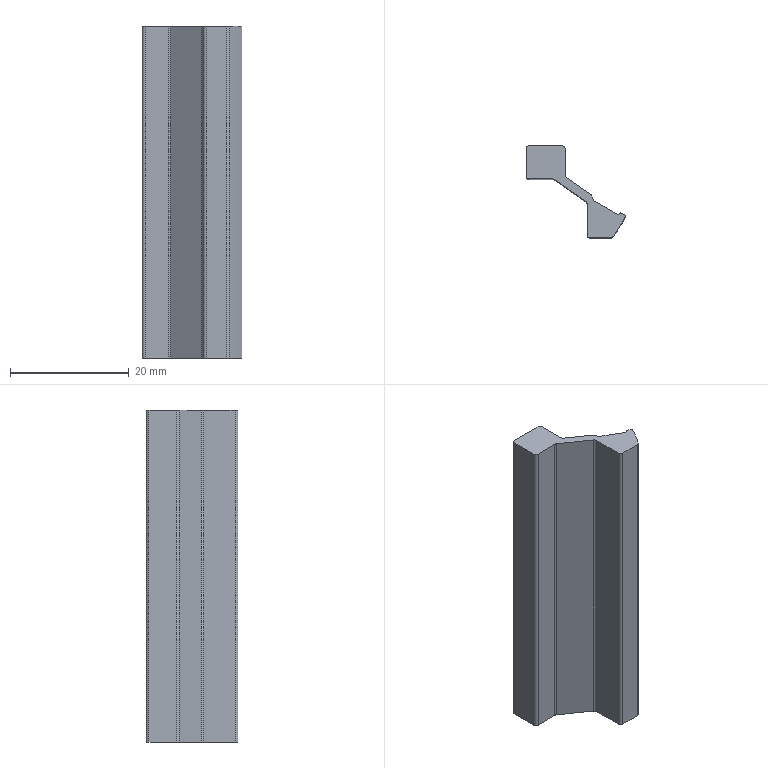Part | NX | features BREP 2 | 2 solids | 50 faces | box 16.849 x 15.507 x 56 mm | volume 8350 mm3 | plane 26 | cylinder 24 | commonest cylinder face diameters 1 x22 72.496 x2
STEP:
#1=CARTESIAN_POINT('',(6.325,-7.535,-4.));
#2=VERTEX_POINT('',#1);
#3=CARTESIAN_POINT('',(6.325,-7.535,52.));
#4=VERTEX_POINT('',#3);
#5=CARTESIAN_POINT('',(6.325,-7.535,0.));
#6=DIRECTION('',(0.,0.,1.));
#7=VECTOR('',#6,1000.);
#8=LINE('',#5,#7);
#9=EDGE_CURVE('',#2,#4,#8,.T.);
#10=ORIENTED_EDGE('',*,*,#9,.T.);
#11=CARTESIAN_POINT('',(5.912,-7.754,52.));
#12=VERTEX_POINT('',#11);
#13=CARTESIAN_POINT('',(5.912,-7.254,52.));
#14=DIRECTION('',(0.,0.,1.));
#15=DIRECTION('',(1.,0.,0.));
#16=AXIS2_PLACEMENT_3D('',#13,#14,#15);
#17=CIRCLE('',#16,0.5);
#18=EDGE_CURVE('',#12,#4,#17,.T.);
#19=ORIENTED_EDGE('',*,*,#18,.F.);
#20=CARTESIAN_POINT('',(5.912,-7.754,-4.));
#21=VERTEX_POINT('',#20);
#22=CARTESIAN_POINT('',(5.912,-7.754,0.));
#23=DIRECTION('',(0.,0.,1.));
#24=VECTOR('',#23,1000.);
#25=LINE('',#22,#24);
#26=EDGE_CURVE('',#21,#12,#25,.T.);
#27=ORIENTED_EDGE('',*,*,#26,.F.);
#28=CARTESIAN_POINT('',(5.912,-7.254,-4.));
#29=DIRECTION('',(0.,0.,1.));
#30=DIRECTION('',(1.,0.,0.));
#31=AXIS2_PLACEMENT_3D('',#28,#29,#30);
#32=CIRCLE('',#31,0.5);
#33=EDGE_CURVE('',#21,#2,#32,.T.);
#34=ORIENTED_EDGE('',*,*,#33,.T.);
#35=EDGE_LOOP('',(#10,#19,#27,#34));
#36=FACE_BOUND('',#35,.T.);
#37=CARTESIAN_POINT('',(5.912,-7.254,0.));
#38=DIRECTION('',(0.,0.,1.));
#39=DIRECTION('',(-1.,0.,0.));
#40=AXIS2_PLACEMENT_3D('',#37,#38,#39);
#41=CYLINDRICAL_SURFACE('',#40,0.5);
#42=ADVANCED_FACE('',(#36),#41,.T.);
#43=ORIENTED_EDGE('',*,*,#26,.T.);
#44=CARTESIAN_POINT('',(2.388,-7.754,52.));
#45=VERTEX_POINT('',#44);
#46=CARTESIAN_POINT('',(-0.3261,-7.754,52.));
#47=DIRECTION('',(1.,0.,0.));
#48=VECTOR('',#47,1000.);
#49=LINE('',#46,#48);
#50=EDGE_CURVE('',#45,#12,#49,.T.);
#51=ORIENTED_EDGE('',*,*,#50,.F.);
#52=CARTESIAN_POINT('',(2.388,-7.754,-4.));
#53=VERTEX_POINT('',#52);
#54=CARTESIAN_POINT('',(2.388,-7.754,0.));
#55=DIRECTION('',(0.,0.,1.));
#56=VECTOR('',#55,1000.);
#57=LINE('',#54,#56);
#58=EDGE_CURVE('',#53,#45,#57,.T.);
#59=ORIENTED_EDGE('',*,*,#58,.F.);
#60=CARTESIAN_POINT('',(-0.3261,-7.754,-4.));
#61=DIRECTION('',(1.,0.,0.));
#62=VECTOR('',#61,1000.);
#63=LINE('',#60,#62);
#64=EDGE_CURVE('',#53,#21,#63,.T.);
#65=ORIENTED_EDGE('',*,*,#64,.T.);
#66=EDGE_LOOP('',(#43,#51,#59,#65));
#67=FACE_BOUND('',#66,.T.);
#68=CARTESIAN_POINT('',(5.912,-7.754,0.));
#69=DIRECTION('',(0.,1.,0.));
#70=DIRECTION('',(1.,0.,0.));
#71=AXIS2_PLACEMENT_3D('',#68,#69,#70);
#72=PLANE('',#71);
#73=ADVANCED_FACE('',(#67),#72,.F.);
#74=ORIENTED_EDGE('',*,*,#58,.T.);
#75=CARTESIAN_POINT('',(1.888,-7.254,52.));
#76=VERTEX_POINT('',#75);
#77=CARTESIAN_POINT('',(2.388,-7.254,52.));
#78=DIRECTION('',(0.,0.,1.));
#79=DIRECTION('',(1.,0.,0.));
#80=AXIS2_PLACEMENT_3D('',#77,#78,#79);
#81=CIRCLE('',#80,0.5);
#82=EDGE_CURVE('',#76,#45,#81,.T.);
#83=ORIENTED_EDGE('',*,*,#82,.F.);
#84=CARTESIAN_POINT('',(1.888,-7.254,-4.));
#85=VERTEX_POINT('',#84);
#86=CARTESIAN_POINT('',(1.888,-7.254,0.));
#87=DIRECTION('',(0.,0.,1.));
#88=VECTOR('',#87,1000.);
#89=LINE('',#86,#88);
#90=EDGE_CURVE('',#85,#76,#89,.T.);
#91=ORIENTED_EDGE('',*,*,#90,.F.);
#92=CARTESIAN_POINT('',(2.388,-7.254,-4.));
#93=DIRECTION('',(0.,0.,1.));
#94=DIRECTION('',(1.,0.,0.));
#95=AXIS2_PLACEMENT_3D('',#92,#93,#94);
#96=CIRCLE('',#95,0.5);
#97=EDGE_CURVE('',#85,#53,#96,.T.);
#98=ORIENTED_EDGE('',*,*,#97,.T.);
#99=EDGE_LOOP('',(#74,#83,#91,#98));
#100=FACE_BOUND('',#99,.T.);
#101=CARTESIAN_POINT('',(2.388,-7.254,0.));
#102=DIRECTION('',(0.,0.,1.));
#103=DIRECTION('',(-1.,0.,0.));
#104=AXIS2_PLACEMENT_3D('',#101,#102,#103);
#105=CYLINDRICAL_SURFACE('',#104,0.5);
#106=ADVANCED_FACE('',(#100),#105,.T.);
#107=ORIENTED_EDGE('',*,*,#90,.T.);
#108=CARTESIAN_POINT('',(1.888,-2.02,52.));
#109=VERTEX_POINT('',#108);
#110=CARTESIAN_POINT('',(1.888,19.254,52.));
#111=DIRECTION('',(0.,-1.,0.));
#112=VECTOR('',#111,1000.);
#113=LINE('',#110,#112);
#114=EDGE_CURVE('',#109,#76,#113,.T.);
#115=ORIENTED_EDGE('',*,*,#114,.F.);
#116=CARTESIAN_POINT('',(1.888,-2.02,-4.));
#117=VERTEX_POINT('',#116);
#118=CARTESIAN_POINT('',(1.888,-2.02,0.));
#119=DIRECTION('',(0.,0.,1.));
#120=VECTOR('',#119,1000.);
#121=LINE('',#118,#120);
#122=EDGE_CURVE('',#117,#109,#121,.T.);
#123=ORIENTED_EDGE('',*,*,#122,.F.);
#124=CARTESIAN_POINT('',(1.888,19.254,-4.));
#125=DIRECTION('',(0.,-1.,0.));
#126=VECTOR('',#125,1000.);
#127=LINE('',#124,#126);
#128=EDGE_CURVE('',#117,#85,#127,.T.);
#129=ORIENTED_EDGE('',*,*,#128,.T.);
#130=EDGE_LOOP('',(#107,#115,#123,#129));
#131=FACE_BOUND('',#130,.T.);
#132=CARTESIAN_POINT('',(1.888,-7.254,0.));
#133=DIRECTION('',(1.,0.,0.));
#134=DIRECTION('',(0.,-1.,0.));
#135=AXIS2_PLACEMENT_3D('',#132,#133,#134);
#136=PLANE('',#135);
#137=ADVANCED_FACE('',(#131),#136,.F.);
#138=ORIENTED_EDGE('',*,*,#122,.T.);
#139=CARTESIAN_POINT('',(1.674,-1.611,52.));
#140=VERTEX_POINT('',#139);
#141=CARTESIAN_POINT('',(1.388,-2.02,52.));
#142=DIRECTION('',(0.,0.,-1.));
#143=DIRECTION('',(1.,0.,0.));
#144=AXIS2_PLACEMENT_3D('',#141,#142,#143);
#145=CIRCLE('',#144,0.5);
#146=EDGE_CURVE('',#140,#109,#145,.T.);
#147=ORIENTED_EDGE('',*,*,#146,.F.);
#148=CARTESIAN_POINT('',(1.674,-1.611,-4.));
#149=VERTEX_POINT('',#148);
#150=CARTESIAN_POINT('',(1.674,-1.611,0.));
#151=DIRECTION('',(0.,0.,1.));
#152=VECTOR('',#151,1000.);
#153=LINE('',#150,#152);
#154=EDGE_CURVE('',#149,#140,#153,.T.);
#155=ORIENTED_EDGE('',*,*,#154,.F.);
#156=CARTESIAN_POINT('',(1.388,-2.02,-4.));
#157=DIRECTION('',(0.,0.,-1.));
#158=DIRECTION('',(1.,0.,0.));
#159=AXIS2_PLACEMENT_3D('',#156,#157,#158);
#160=CIRCLE('',#159,0.5);
#161=EDGE_CURVE('',#149,#117,#160,.T.);
#162=ORIENTED_EDGE('',*,*,#161,.T.);
#163=EDGE_LOOP('',(#138,#147,#155,#162));
#164=FACE_BOUND('',#163,.T.);
#165=CARTESIAN_POINT('',(1.388,-2.02,0.));
#166=DIRECTION('',(0.,0.,1.));
#167=DIRECTION('',(-1.,0.,0.));
#168=AXIS2_PLACEMENT_3D('',#165,#166,#167);
#169=CYLINDRICAL_SURFACE('',#168,0.5);
#170=ADVANCED_FACE('',(#164),#169,.F.);
#171=ORIENTED_EDGE('',*,*,#154,.T.);
#172=CARTESIAN_POINT('',(-3.57,2.062,52.));
#173=VERTEX_POINT('',#172);
#174=CARTESIAN_POINT('',(1.674,-1.611,52.));
#175=DIRECTION('',(0.8192,-0.5736,0.));
#176=VECTOR('',#175,1000.);
#177=LINE('',#174,#176);
#178=EDGE_CURVE('',#173,#140,#177,.T.);
#179=ORIENTED_EDGE('',*,*,#178,.F.);
#180=CARTESIAN_POINT('',(-3.57,2.062,-4.));
#181=VERTEX_POINT('',#180);
#182=CARTESIAN_POINT('',(-3.57,2.062,0.));
#183=DIRECTION('',(0.,0.,1.));
#184=VECTOR('',#183,1000.);
#185=LINE('',#182,#184);
#186=EDGE_CURVE('',#181,#173,#185,.T.);
#187=ORIENTED_EDGE('',*,*,#186,.F.);
#188=CARTESIAN_POINT('',(1.674,-1.611,-4.));
#189=DIRECTION('',(0.8192,-0.5736,0.));
#190=VECTOR('',#189,1000.);
#191=LINE('',#188,#190);
#192=EDGE_CURVE('',#181,#149,#191,.T.);
#193=ORIENTED_EDGE('',*,*,#192,.T.);
#194=EDGE_LOOP('',(#171,#179,#187,#193));
#195=FACE_BOUND('',#194,.T.);
#196=CARTESIAN_POINT('',(1.674,-1.611,0.));
#197=DIRECTION('',(0.5736,0.8192,0.));
#198=DIRECTION('',(0.8192,-0.5736,0.));
#199=AXIS2_PLACEMENT_3D('',#196,#197,#198);
#200=PLANE('',#199);
#201=ADVANCED_FACE('',(#195),#200,.F.);
#202=ORIENTED_EDGE('',*,*,#186,.T.);
#203=CARTESIAN_POINT('',(-3.857,2.152,52.));
#204=VERTEX_POINT('',#203);
#205=CARTESIAN_POINT('',(-3.857,1.652,52.));
#206=DIRECTION('',(0.,0.,-1.));
#207=DIRECTION('',(1.,0.,0.));
#208=AXIS2_PLACEMENT_3D('',#205,#206,#207);
#209=CIRCLE('',#208,0.5);
#210=EDGE_CURVE('',#204,#173,#209,.T.);
#211=ORIENTED_EDGE('',*,*,#210,.F.);
#212=CARTESIAN_POINT('',(-3.857,2.152,-4.));
#213=VERTEX_POINT('',#212);
#214=CARTESIAN_POINT('',(-3.857,2.152,0.));
#215=DIRECTION('',(0.,0.,1.));
#216=VECTOR('',#215,1000.);
#217=LINE('',#214,#216);
#218=EDGE_CURVE('',#213,#204,#217,.T.);
#219=ORIENTED_EDGE('',*,*,#218,.F.);
#220=CARTESIAN_POINT('',(-3.857,1.652,-4.));
#221=DIRECTION('',(0.,0.,-1.));
#222=DIRECTION('',(1.,0.,0.));
#223=AXIS2_PLACEMENT_3D('',#220,#221,#222);
#224=CIRCLE('',#223,0.5);
#225=EDGE_CURVE('',#213,#181,#224,.T.);
#226=ORIENTED_EDGE('',*,*,#225,.T.);
#227=EDGE_LOOP('',(#202,#211,#219,#226));
#228=FACE_BOUND('',#227,.T.);
#229=CARTESIAN_POINT('',(-3.857,1.652,0.));
#230=DIRECTION('',(0.,0.,1.));
#231=DIRECTION('',(-1.,0.,0.));
#232=AXIS2_PLACEMENT_3D('',#229,#230,#231);
#233=CYLINDRICAL_SURFACE('',#232,0.5);
#234=ADVANCED_FACE('',(#228),#233,.F.);
#235=ORIENTED_EDGE('',*,*,#218,.T.);
#236=CARTESIAN_POINT('',(-7.9,2.152,52.));
#237=VERTEX_POINT('',#236);
#238=CARTESIAN_POINT('',(-0.3261,2.152,52.));
#239=DIRECTION('',(1.,0.,0.));
#240=VECTOR('',#239,1000.);
#241=LINE('',#238,#240);
#242=EDGE_CURVE('',#237,#204,#241,.T.);
#243=ORIENTED_EDGE('',*,*,#242,.F.);
#244=CARTESIAN_POINT('',(-7.9,2.152,-4.));
#245=VERTEX_POINT('',#244);
#246=CARTESIAN_POINT('',(-7.9,2.152,0.));
#247=DIRECTION('',(0.,0.,1.));
#248=VECTOR('',#247,1000.);
#249=LINE('',#246,#248);
#250=EDGE_CURVE('',#245,#237,#249,.T.);
#251=ORIENTED_EDGE('',*,*,#250,.F.);
#252=CARTESIAN_POINT('',(-0.3261,2.152,-4.));
#253=DIRECTION('',(1.,0.,0.));
#254=VECTOR('',#253,1000.);
#255=LINE('',#252,#254);
#256=EDGE_CURVE('',#245,#213,#255,.T.);
#257=ORIENTED_EDGE('',*,*,#256,.T.);
#258=EDGE_LOOP('',(#235,#243,#251,#257));
#259=FACE_BOUND('',#258,.T.);
#260=CARTESIAN_POINT('',(-3.857,2.152,0.));
#261=DIRECTION('',(0.,1.,0.));
#262=DIRECTION('',(1.,0.,0.));
#263=AXIS2_PLACEMENT_3D('',#260,#261,#262);
#264=PLANE('',#263);
#265=ADVANCED_FACE('',(#259),#264,.F.);
#266=ORIENTED_EDGE('',*,*,#250,.T.);
#267=CARTESIAN_POINT('',(-8.4,2.652,52.));
#268=VERTEX_POINT('',#267);
#269=CARTESIAN_POINT('',(-7.9,2.652,52.));
#270=DIRECTION('',(0.,0.,1.));
#271=DIRECTION('',(1.,0.,0.));
#272=AXIS2_PLACEMENT_3D('',#269,#270,#271);
#273=CIRCLE('',#272,0.5);
#274=EDGE_CURVE('',#268,#237,#273,.T.);
#275=ORIENTED_EDGE('',*,*,#274,.F.);
#276=CARTESIAN_POINT('',(-8.4,2.652,-4.));
#277=VERTEX_POINT('',#276);
#278=CARTESIAN_POINT('',(-8.4,2.652,0.));
#279=DIRECTION('',(0.,0.,1.));
#280=VECTOR('',#279,1000.);
#281=LINE('',#278,#280);
#282=EDGE_CURVE('',#277,#268,#281,.T.);
#283=ORIENTED_EDGE('',*,*,#282,.F.);
#284=CARTESIAN_POINT('',(-7.9,2.652,-4.));
#285=DIRECTION('',(0.,0.,1.));
#286=DIRECTION('',(1.,0.,0.));
#287=AXIS2_PLACEMENT_3D('',#284,#285,#286);
#288=CIRCLE('',#287,0.5);
#289=EDGE_CURVE('',#277,#245,#288,.T.);
#290=ORIENTED_EDGE('',*,*,#289,.T.);
#291=EDGE_LOOP('',(#266,#275,#283,#290));
#292=FACE_BOUND('',#291,.T.);
#293=CARTESIAN_POINT('',(-7.9,2.652,0.));
#294=DIRECTION('',(0.,0.,1.));
#295=DIRECTION('',(-1.,0.,0.));
#296=AXIS2_PLACEMENT_3D('',#293,#294,#295);
#297=CYLINDRICAL_SURFACE('',#296,0.5);
#298=ADVANCED_FACE('',(#292),#297,.T.);
#299=ORIENTED_EDGE('',*,*,#282,.T.);
#300=CARTESIAN_POINT('',(-8.4,7.254,52.));
#301=VERTEX_POINT('',#300);
#302=CARTESIAN_POINT('',(-8.4,19.254,52.));
#303=DIRECTION('',(0.,-1.,0.));
#304=VECTOR('',#303,1000.);
#305=LINE('',#302,#304);
#306=EDGE_CURVE('',#301,#268,#305,.T.);
#307=ORIENTED_EDGE('',*,*,#306,.F.);
#308=CARTESIAN_POINT('',(-8.4,7.254,-4.));
#309=VERTEX_POINT('',#308);
#310=CARTESIAN_POINT('',(-8.4,7.254,0.));
#311=DIRECTION('',(0.,0.,1.));
#312=VECTOR('',#311,1000.);
#313=LINE('',#310,#312);
#314=EDGE_CURVE('',#309,#301,#313,.T.);
#315=ORIENTED_EDGE('',*,*,#314,.F.);
#316=CARTESIAN_POINT('',(-8.4,19.254,-4.));
#317=DIRECTION('',(0.,-1.,0.));
#318=VECTOR('',#317,1000.);
#319=LINE('',#316,#318);
#320=EDGE_CURVE('',#309,#277,#319,.T.);
#321=ORIENTED_EDGE('',*,*,#320,.T.);
#322=EDGE_LOOP('',(#299,#307,#315,#321));
#323=FACE_BOUND('',#322,.T.);
#324=CARTESIAN_POINT('',(-8.4,2.652,0.));
#325=DIRECTION('',(1.,0.,0.));
#326=DIRECTION('',(0.,-1.,0.));
#327=AXIS2_PLACEMENT_3D('',#324,#325,#326);
#328=PLANE('',#327);
#329=ADVANCED_FACE('',(#323),#328,.F.);
#330=ORIENTED_EDGE('',*,*,#314,.T.);
#331=CARTESIAN_POINT('',(-7.9,7.754,52.));
#332=VERTEX_POINT('',#331);
#333=CARTESIAN_POINT('',(-7.9,7.254,52.));
#334=DIRECTION('',(0.,0.,1.));
#335=DIRECTION('',(1.,0.,0.));
#336=AXIS2_PLACEMENT_3D('',#333,#334,#335);
#337=CIRCLE('',#336,0.5);
#338=EDGE_CURVE('',#332,#301,#337,.T.);
#339=ORIENTED_EDGE('',*,*,#338,.F.);
#340=CARTESIAN_POINT('',(-7.9,7.754,-4.));
#341=VERTEX_POINT('',#340);
#342=CARTESIAN_POINT('',(-7.9,7.754,0.));
#343=DIRECTION('',(0.,0.,1.));
#344=VECTOR('',#343,1000.);
#345=LINE('',#342,#344);
#346=EDGE_CURVE('',#341,#332,#345,.T.);
#347=ORIENTED_EDGE('',*,*,#346,.F.);
#348=CARTESIAN_POINT('',(-7.9,7.254,-4.));
#349=DIRECTION('',(0.,0.,1.));
#350=DIRECTION('',(1.,0.,0.));
#351=AXIS2_PLACEMENT_3D('',#348,#349,#350);
#352=CIRCLE('',#351,0.5);
#353=EDGE_CURVE('',#341,#309,#352,.T.);
#354=ORIENTED_EDGE('',*,*,#353,.T.);
#355=EDGE_LOOP('',(#330,#339,#347,#354));
#356=FACE_BOUND('',#355,.T.);
#357=CARTESIAN_POINT('',(-7.9,7.254,0.));
#358=DIRECTION('',(0.,0.,1.));
#359=DIRECTION('',(-1.,0.,0.));
#360=AXIS2_PLACEMENT_3D('',#357,#358,#359);
#361=CYLINDRICAL_SURFACE('',#360,0.5);
#362=ADVANCED_FACE('',(#356),#361,.T.);
#363=ORIENTED_EDGE('',*,*,#346,.T.);
#364=CARTESIAN_POINT('',(-2.3,7.754,52.));
#365=VERTEX_POINT('',#364);
#366=CARTESIAN_POINT('',(-0.3261,7.754,52.));
#367=DIRECTION('',(-1.,0.,0.));
#368=VECTOR('',#367,1000.);
#369=LINE('',#366,#368);
#370=EDGE_CURVE('',#365,#332,#369,.T.);
#371=ORIENTED_EDGE('',*,*,#370,.F.);
#372=CARTESIAN_POINT('',(-2.3,7.754,-4.));
#373=VERTEX_POINT('',#372);
#374=CARTESIAN_POINT('',(-2.3,7.754,0.));
#375=DIRECTION('',(0.,0.,1.));
#376=VECTOR('',#375,1000.);
#377=LINE('',#374,#376);
#378=EDGE_CURVE('',#373,#365,#377,.T.);
#379=ORIENTED_EDGE('',*,*,#378,.F.);
#380=CARTESIAN_POINT('',(-0.3261,7.754,-4.));
#381=DIRECTION('',(-1.,0.,0.));
#382=VECTOR('',#381,1000.);
#383=LINE('',#380,#382);
#384=EDGE_CURVE('',#373,#341,#383,.T.);
#385=ORIENTED_EDGE('',*,*,#384,.T.);
#386=EDGE_LOOP('',(#363,#371,#379,#385));
#387=FACE_BOUND('',#386,.T.);
#388=CARTESIAN_POINT('',(-7.9,7.754,0.));
#389=DIRECTION('',(0.,-1.,0.));
#390=DIRECTION('',(-1.,0.,0.));
#391=AXIS2_PLACEMENT_3D('',#388,#389,#390);
#392=PLANE('',#391);
#393=ADVANCED_FACE('',(#387),#392,.F.);
#394=ORIENTED_EDGE('',*,*,#378,.T.);
#395=CARTESIAN_POINT('',(-1.8,7.254,52.));
#396=VERTEX_POINT('',#395);
#397=CARTESIAN_POINT('',(-2.3,7.254,52.));
#398=DIRECTION('',(0.,0.,1.));
#399=DIRECTION('',(1.,0.,0.));
#400=AXIS2_PLACEMENT_3D('',#397,#398,#399);
#401=CIRCLE('',#400,0.5);
#402=EDGE_CURVE('',#396,#365,#401,.T.);
#403=ORIENTED_EDGE('',*,*,#402,.F.);
#404=CARTESIAN_POINT('',(-1.8,7.254,-4.));
#405=VERTEX_POINT('',#404);
#406=CARTESIAN_POINT('',(-1.8,7.254,0.));
#407=DIRECTION('',(0.,0.,1.));
#408=VECTOR('',#407,1000.);
#409=LINE('',#406,#408);
#410=EDGE_CURVE('',#405,#396,#409,.T.);
#411=ORIENTED_EDGE('',*,*,#410,.F.);
#412=CARTESIAN_POINT('',(-2.3,7.254,-4.));
#413=DIRECTION('',(0.,0.,1.));
#414=DIRECTION('',(1.,0.,0.));
#415=AXIS2_PLACEMENT_3D('',#412,#413,#414);
#416=CIRCLE('',#415,0.5);
#417=EDGE_CURVE('',#405,#373,#416,.T.);
#418=ORIENTED_EDGE('',*,*,#417,.T.);
#419=EDGE_LOOP('',(#394,#403,#411,#418));
#420=FACE_BOUND('',#419,.T.);
#421=CARTESIAN_POINT('',(-2.3,7.254,0.));
#422=DIRECTION('',(0.,0.,1.));
#423=DIRECTION('',(-1.,0.,0.));
#424=AXIS2_PLACEMENT_3D('',#421,#422,#423);
#425=CYLINDRICAL_SURFACE('',#424,0.5);
#426=ADVANCED_FACE('',(#420),#425,.T.);
#427=ORIENTED_EDGE('',*,*,#410,.T.);
#428=CARTESIAN_POINT('',(-1.8,2.814,52.));
#429=VERTEX_POINT('',#428);
#430=CARTESIAN_POINT('',(-1.8,19.254,52.));
#431=DIRECTION('',(0.,1.,0.));
#432=VECTOR('',#431,1000.);
#433=LINE('',#430,#432);
#434=EDGE_CURVE('',#429,#396,#433,.T.);
#435=ORIENTED_EDGE('',*,*,#434,.F.);
#436=CARTESIAN_POINT('',(-1.8,2.814,-4.));
#437=VERTEX_POINT('',#436);
#438=CARTESIAN_POINT('',(-1.8,2.814,0.));
#439=DIRECTION('',(0.,0.,1.));
#440=VECTOR('',#439,1000.);
#441=LINE('',#438,#440);
#442=EDGE_CURVE('',#437,#429,#441,.T.);
#443=ORIENTED_EDGE('',*,*,#442,.F.);
#444=CARTESIAN_POINT('',(-1.8,19.254,-4.));
#445=DIRECTION('',(0.,1.,0.));
#446=VECTOR('',#445,1000.);
#447=LINE('',#444,#446);
#448=EDGE_CURVE('',#437,#405,#447,.T.);
#449=ORIENTED_EDGE('',*,*,#448,.T.);
#450=EDGE_LOOP('',(#427,#435,#443,#449));
#451=FACE_BOUND('',#450,.T.);
#452=CARTESIAN_POINT('',(-1.8,7.254,0.));
#453=DIRECTION('',(-1.,0.,0.));
#454=DIRECTION('',(0.,1.,0.));
#455=AXIS2_PLACEMENT_3D('',#452,#453,#454);
#456=PLANE('',#455);
#457=ADVANCED_FACE('',(#451),#456,.F.);
#458=ORIENTED_EDGE('',*,*,#442,.T.);
#459=CARTESIAN_POINT('',(-1.586,2.404,52.));
#460=VERTEX_POINT('',#459);
#461=CARTESIAN_POINT('',(-1.3,2.814,52.));
#462=DIRECTION('',(0.,0.,-1.));
#463=DIRECTION('',(1.,0.,0.));
#464=AXIS2_PLACEMENT_3D('',#461,#462,#463);
#465=CIRCLE('',#464,0.5);
#466=EDGE_CURVE('',#460,#429,#465,.T.);
#467=ORIENTED_EDGE('',*,*,#466,.F.);
#468=CARTESIAN_POINT('',(-1.586,2.404,-4.));
#469=VERTEX_POINT('',#468);
#470=CARTESIAN_POINT('',(-1.586,2.404,0.));
#471=DIRECTION('',(0.,0.,1.));
#472=VECTOR('',#471,1000.);
#473=LINE('',#470,#472);
#474=EDGE_CURVE('',#469,#460,#473,.T.);
#475=ORIENTED_EDGE('',*,*,#474,.F.);
#476=CARTESIAN_POINT('',(-1.3,2.814,-4.));
#477=DIRECTION('',(0.,0.,-1.));
#478=DIRECTION('',(1.,0.,0.));
#479=AXIS2_PLACEMENT_3D('',#476,#477,#478);
#480=CIRCLE('',#479,0.5);
#481=EDGE_CURVE('',#469,#437,#480,.T.);
#482=ORIENTED_EDGE('',*,*,#481,.T.);
#483=EDGE_LOOP('',(#458,#467,#475,#482));
#484=FACE_BOUND('',#483,.T.);
#485=CARTESIAN_POINT('',(-1.3,2.814,0.));
#486=DIRECTION('',(0.,0.,1.));
#487=DIRECTION('',(-1.,0.,0.));
#488=AXIS2_PLACEMENT_3D('',#485,#486,#487);
#489=CYLINDRICAL_SURFACE('',#488,0.5);
#490=ADVANCED_FACE('',(#484),#489,.F.);
#491=ORIENTED_EDGE('',*,*,#474,.T.);
#492=CARTESIAN_POINT('',(2.495,-0.4532,52.));
#493=VERTEX_POINT('',#492);
#494=CARTESIAN_POINT('',(-1.586,2.404,52.));
#495=DIRECTION('',(-0.8192,0.5736,0.));
#496=VECTOR('',#495,1000.);
#497=LINE('',#494,#496);
#498=EDGE_CURVE('',#493,#460,#497,.T.);
#499=ORIENTED_EDGE('',*,*,#498,.F.);
#500=CARTESIAN_POINT('',(2.495,-0.4532,-4.));
#501=VERTEX_POINT('',#500);
#502=CARTESIAN_POINT('',(2.495,-0.4532,0.));
#503=DIRECTION('',(0.,0.,1.));
#504=VECTOR('',#503,1000.);
#505=LINE('',#502,#504);
#506=EDGE_CURVE('',#501,#493,#505,.T.);
#507=ORIENTED_EDGE('',*,*,#506,.F.);
#508=CARTESIAN_POINT('',(-1.586,2.404,-4.));
#509=DIRECTION('',(-0.8192,0.5736,0.));
#510=VECTOR('',#509,1000.);
#511=LINE('',#508,#510);
#512=EDGE_CURVE('',#501,#469,#511,.T.);
#513=ORIENTED_EDGE('',*,*,#512,.T.);
#514=EDGE_LOOP('',(#491,#499,#507,#513));
#515=FACE_BOUND('',#514,.T.);
#516=CARTESIAN_POINT('',(-1.586,2.404,0.));
#517=DIRECTION('',(-0.5736,-0.8192,0.));
#518=DIRECTION('',(-0.8192,0.5736,0.));
#519=AXIS2_PLACEMENT_3D('',#516,#517,#518);
#520=PLANE('',#519);
#521=ADVANCED_FACE('',(#515),#520,.F.);
#522=ORIENTED_EDGE('',*,*,#506,.T.);
#523=CARTESIAN_POINT('',(2.678,-0.6918,52.));
#524=VERTEX_POINT('',#523);
#525=CARTESIAN_POINT('',(2.208,-0.8628,52.));
#526=DIRECTION('',(0.,0.,1.));
#527=DIRECTION('',(1.,0.,0.));
#528=AXIS2_PLACEMENT_3D('',#525,#526,#527);
#529=CIRCLE('',#528,0.5);
#530=EDGE_CURVE('',#524,#493,#529,.T.);
#531=ORIENTED_EDGE('',*,*,#530,.F.);
#532=CARTESIAN_POINT('',(2.678,-0.6918,-4.));
#533=VERTEX_POINT('',#532);
#534=CARTESIAN_POINT('',(2.678,-0.6918,0.));
#535=DIRECTION('',(0.,0.,1.));
#536=VECTOR('',#535,1000.);
#537=LINE('',#534,#536);
#538=EDGE_CURVE('',#533,#524,#537,.T.);
#539=ORIENTED_EDGE('',*,*,#538,.F.);
#540=CARTESIAN_POINT('',(2.208,-0.8628,-4.));
#541=DIRECTION('',(0.,0.,1.));
#542=DIRECTION('',(1.,0.,0.));
#543=AXIS2_PLACEMENT_3D('',#540,#541,#542);
#544=CIRCLE('',#543,0.5);
#545=EDGE_CURVE('',#533,#501,#544,.T.);
#546=ORIENTED_EDGE('',*,*,#545,.T.);
#547=EDGE_LOOP('',(#522,#531,#539,#546));
#548=FACE_BOUND('',#547,.T.);
#549=CARTESIAN_POINT('',(2.208,-0.8628,0.));
#550=DIRECTION('',(0.,0.,1.));
#551=DIRECTION('',(-1.,0.,0.));
#552=AXIS2_PLACEMENT_3D('',#549,#550,#551);
#553=CYLINDRICAL_SURFACE('',#552,0.5);
#554=ADVANCED_FACE('',(#548),#553,.T.);
#555=ORIENTED_EDGE('',*,*,#538,.T.);
#556=CARTESIAN_POINT('',(2.904,-1.312,52.));
#557=VERTEX_POINT('',#556);
#558=CARTESIAN_POINT('',(2.678,-0.6918,52.));
#559=DIRECTION('',(-0.342,0.9397,0.));
#560=VECTOR('',#559,1000.);
#561=LINE('',#558,#560);
#562=EDGE_CURVE('',#557,#524,#561,.T.);
#563=ORIENTED_EDGE('',*,*,#562,.F.);
#564=CARTESIAN_POINT('',(2.904,-1.312,-4.));
#565=VERTEX_POINT('',#564);
#566=CARTESIAN_POINT('',(2.904,-1.312,0.));
#567=DIRECTION('',(0.,0.,1.));
#568=VECTOR('',#567,1000.);
#569=LINE('',#566,#568);
#570=EDGE_CURVE('',#565,#557,#569,.T.);
#571=ORIENTED_EDGE('',*,*,#570,.F.);
#572=CARTESIAN_POINT('',(2.678,-0.6918,-4.));
#573=DIRECTION('',(-0.342,0.9397,0.));
#574=VECTOR('',#573,1000.);
#575=LINE('',#572,#574);
#576=EDGE_CURVE('',#565,#533,#575,.T.);
#577=ORIENTED_EDGE('',*,*,#576,.T.);
#578=EDGE_LOOP('',(#555,#563,#571,#577));
#579=FACE_BOUND('',#578,.T.);
#580=CARTESIAN_POINT('',(2.678,-0.6918,0.));
#581=DIRECTION('',(-0.9397,-0.342,0.));
#582=DIRECTION('',(-0.342,0.9397,0.));
#583=AXIS2_PLACEMENT_3D('',#580,#581,#582);
#584=PLANE('',#583);
#585=ADVANCED_FACE('',(#579),#584,.F.);
#586=ORIENTED_EDGE('',*,*,#570,.T.);
#587=CARTESIAN_POINT('',(3.123,-1.574,52.));
#588=VERTEX_POINT('',#587);
#589=CARTESIAN_POINT('',(3.373,-1.141,52.));
#590=DIRECTION('',(0.,0.,-1.));
#591=DIRECTION('',(1.,0.,0.));
#592=AXIS2_PLACEMENT_3D('',#589,#590,#591);
#593=CIRCLE('',#592,0.5);
#594=EDGE_CURVE('',#588,#557,#593,.T.);
#595=ORIENTED_EDGE('',*,*,#594,.F.);
#596=CARTESIAN_POINT('',(3.123,-1.574,-4.));
#597=VERTEX_POINT('',#596);
#598=CARTESIAN_POINT('',(3.123,-1.574,0.));
#599=DIRECTION('',(0.,0.,1.));
#600=VECTOR('',#599,1000.);
#601=LINE('',#598,#600);
#602=EDGE_CURVE('',#597,#588,#601,.T.);
#603=ORIENTED_EDGE('',*,*,#602,.F.);
#604=CARTESIAN_POINT('',(3.373,-1.141,-4.));
#605=DIRECTION('',(0.,0.,-1.));
#606=DIRECTION('',(1.,0.,0.));
#607=AXIS2_PLACEMENT_3D('',#604,#605,#606);
#608=CIRCLE('',#607,0.5);
#609=EDGE_CURVE('',#597,#565,#608,.T.);
#610=ORIENTED_EDGE('',*,*,#609,.T.);
#611=EDGE_LOOP('',(#586,#595,#603,#610));
#612=FACE_BOUND('',#611,.T.);
#613=CARTESIAN_POINT('',(3.373,-1.141,0.));
#614=DIRECTION('',(0.,0.,1.));
#615=DIRECTION('',(-1.,0.,0.));
#616=AXIS2_PLACEMENT_3D('',#613,#614,#615);
#617=CYLINDRICAL_SURFACE('',#616,0.5);
#618=ADVANCED_FACE('',(#612),#617,.F.);
#619=ORIENTED_EDGE('',*,*,#602,.T.);
#620=CARTESIAN_POINT('',(6.845,-3.723,52.));
#621=VERTEX_POINT('',#620);
#622=CARTESIAN_POINT('',(3.123,-1.574,52.));
#623=DIRECTION('',(-0.866,0.5,0.));
#624=VECTOR('',#623,1000.);
#625=LINE('',#622,#624);
#626=EDGE_CURVE('',#621,#588,#625,.T.);
#627=ORIENTED_EDGE('',*,*,#626,.F.);
#628=CARTESIAN_POINT('',(6.845,-3.723,-4.));
#629=VERTEX_POINT('',#628);
#630=CARTESIAN_POINT('',(6.845,-3.723,0.));
#631=DIRECTION('',(0.,0.,1.));
#632=VECTOR('',#631,1000.);
#633=LINE('',#630,#632);
#634=EDGE_CURVE('',#629,#621,#633,.T.);
#635=ORIENTED_EDGE('',*,*,#634,.F.);
#636=CARTESIAN_POINT('',(3.123,-1.574,-4.));
#637=DIRECTION('',(-0.866,0.5,0.));
#638=VECTOR('',#637,1000.);
#639=LINE('',#636,#638);
#640=EDGE_CURVE('',#629,#597,#639,.T.);
#641=ORIENTED_EDGE('',*,*,#640,.T.);
#642=EDGE_LOOP('',(#619,#627,#635,#641));
#643=FACE_BOUND('',#642,.T.);
#644=CARTESIAN_POINT('',(3.123,-1.574,0.));
#645=DIRECTION('',(-0.5,-0.866,0.));
#646=DIRECTION('',(-0.866,0.5,0.));
#647=AXIS2_PLACEMENT_3D('',#644,#645,#646);
#648=PLANE('',#647);
#649=ADVANCED_FACE('',(#643),#648,.F.);
#650=ORIENTED_EDGE('',*,*,#634,.T.);
#651=CARTESIAN_POINT('',(7.539,-3.518,52.));
#652=VERTEX_POINT('',#651);
#653=CARTESIAN_POINT('',(7.095,-3.29,52.));
#654=DIRECTION('',(0.,0.,-1.));
#655=DIRECTION('',(1.,0.,0.));
#656=AXIS2_PLACEMENT_3D('',#653,#654,#655);
#657=CIRCLE('',#656,0.5);
#658=EDGE_CURVE('',#652,#621,#657,.T.);
#659=ORIENTED_EDGE('',*,*,#658,.F.);
#660=CARTESIAN_POINT('',(7.539,-3.518,-4.));
#661=VERTEX_POINT('',#660);
#662=CARTESIAN_POINT('',(7.539,-3.518,0.));
#663=DIRECTION('',(0.,0.,1.));
#664=VECTOR('',#663,1000.);
#665=LINE('',#662,#664);
#666=EDGE_CURVE('',#661,#652,#665,.T.);
#667=ORIENTED_EDGE('',*,*,#666,.F.);
#668=CARTESIAN_POINT('',(7.095,-3.29,-4.));
#669=DIRECTION('',(0.,0.,-1.));
#670=DIRECTION('',(1.,0.,0.));
#671=AXIS2_PLACEMENT_3D('',#668,#669,#670);
#672=CIRCLE('',#671,0.5);
#673=EDGE_CURVE('',#661,#629,#672,.T.);
#674=ORIENTED_EDGE('',*,*,#673,.T.);
#675=EDGE_LOOP('',(#650,#659,#667,#674));
#676=FACE_BOUND('',#675,.T.);
#677=CARTESIAN_POINT('',(7.095,-3.29,0.));
#678=DIRECTION('',(0.,0.,1.));
#679=DIRECTION('',(-1.,0.,0.));
#680=AXIS2_PLACEMENT_3D('',#677,#678,#679);
#681=CYLINDRICAL_SURFACE('',#680,0.5);
#682=ADVANCED_FACE('',(#676),#681,.F.);
#683=ORIENTED_EDGE('',*,*,#666,.T.);
#684=CARTESIAN_POINT('',(8.45,-3.996,52.));
#685=VERTEX_POINT('',#684);
#686=CARTESIAN_POINT('',(-8.001,4.647,52.));
#687=DIRECTION('',(-0.8853,0.4651,0.));
#688=VECTOR('',#687,1000.);
#689=LINE('',#686,#688);
#690=EDGE_CURVE('',#685,#652,#689,.T.);
#691=ORIENTED_EDGE('',*,*,#690,.F.);
#692=CARTESIAN_POINT('',(8.45,-3.996,-4.));
#693=VERTEX_POINT('',#692);
#694=CARTESIAN_POINT('',(8.45,-3.996,0.));
#695=DIRECTION('',(0.,0.,1.));
#696=VECTOR('',#695,1000.);
#697=LINE('',#694,#696);
#698=EDGE_CURVE('',#693,#685,#697,.T.);
#699=ORIENTED_EDGE('',*,*,#698,.F.);
#700=CARTESIAN_POINT('',(-8.001,4.647,-4.));
#701=DIRECTION('',(-0.8853,0.4651,0.));
#702=VECTOR('',#701,1000.);
#703=LINE('',#700,#702);
#704=EDGE_CURVE('',#693,#661,#703,.T.);
#705=ORIENTED_EDGE('',*,*,#704,.T.);
#706=EDGE_LOOP('',(#683,#691,#699,#705));
#707=FACE_BOUND('',#706,.T.);
#708=CARTESIAN_POINT('',(-8.001,4.647,0.));
#709=DIRECTION('',(-0.4651,-0.8853,0.));
#710=DIRECTION('',(-0.8853,0.4651,0.));
#711=AXIS2_PLACEMENT_3D('',#708,#709,#710);
#712=PLANE('',#711);
#713=ADVANCED_FACE('',(#707),#712,.F.);
#714=CARTESIAN_POINT('',(-23.639,12.863,-4.));
#715=DIRECTION('',(0.,0.,1.));
#716=DIRECTION('',(1.,0.,0.));
#717=AXIS2_PLACEMENT_3D('',#714,#715,#716);
#718=CIRCLE('',#717,36.248);
#719=EDGE_CURVE('',#2,#693,#718,.T.);
#720=ORIENTED_EDGE('',*,*,#719,.T.);
#721=ORIENTED_EDGE('',*,*,#698,.T.);
#722=CARTESIAN_POINT('',(-23.639,12.863,52.));
#723=DIRECTION('',(0.,0.,1.));
#724=DIRECTION('',(1.,0.,0.));
#725=AXIS2_PLACEMENT_3D('',#722,#723,#724);
#726=CIRCLE('',#725,36.248);
#727=EDGE_CURVE('',#4,#685,#726,.T.);
#728=ORIENTED_EDGE('',*,*,#727,.F.);
#729=ORIENTED_EDGE('',*,*,#9,.F.);
#730=EDGE_LOOP('',(#720,#721,#728,#729));
#731=FACE_BOUND('',#730,.T.);
#732=CARTESIAN_POINT('',(-23.639,12.863,0.));
#733=DIRECTION('',(0.,0.,1.));
#734=DIRECTION('',(-1.,0.,0.));
#735=AXIS2_PLACEMENT_3D('',#732,#733,#734);
#736=CYLINDRICAL_SURFACE('',#735,36.248);
#737=ADVANCED_FACE('',(#731),#736,.T.);
#738=ORIENTED_EDGE('',*,*,#690,.T.);
#739=ORIENTED_EDGE('',*,*,#658,.T.);
#740=ORIENTED_EDGE('',*,*,#626,.T.);
#741=ORIENTED_EDGE('',*,*,#594,.T.);
#742=ORIENTED_EDGE('',*,*,#562,.T.);
#743=ORIENTED_EDGE('',*,*,#530,.T.);
#744=ORIENTED_EDGE('',*,*,#498,.T.);
#745=ORIENTED_EDGE('',*,*,#466,.T.);
#746=ORIENTED_EDGE('',*,*,#434,.T.);
#747=ORIENTED_EDGE('',*,*,#402,.T.);
#748=ORIENTED_EDGE('',*,*,#370,.T.);
#749=ORIENTED_EDGE('',*,*,#338,.T.);
#750=ORIENTED_EDGE('',*,*,#306,.T.);
#751=ORIENTED_EDGE('',*,*,#274,.T.);
#752=ORIENTED_EDGE('',*,*,#242,.T.);
#753=ORIENTED_EDGE('',*,*,#210,.T.);
#754=ORIENTED_EDGE('',*,*,#178,.T.);
#755=ORIENTED_EDGE('',*,*,#146,.T.);
#756=ORIENTED_EDGE('',*,*,#114,.T.);
#757=ORIENTED_EDGE('',*,*,#82,.T.);
#758=ORIENTED_EDGE('',*,*,#50,.T.);
#759=ORIENTED_EDGE('',*,*,#18,.T.);
#760=ORIENTED_EDGE('',*,*,#727,.T.);
#761=EDGE_LOOP('',(#738,#739,#740,#741,#742,#743,#744,#745,#746,#747,#748,#749,#750,#751,#752,#753,#754,#755,#756,#757,#758,#759,#760));
#762=FACE_BOUND('',#761,.T.);
#763=CARTESIAN_POINT('',(-0.3261,19.254,52.));
#764=DIRECTION('',(0.,0.,1.));
#765=DIRECTION('',(-1.,0.,0.));
#766=AXIS2_PLACEMENT_3D('',#763,#764,#765);
#767=PLANE('',#766);
#768=ADVANCED_FACE('',(#762),#767,.T.);
#769=ORIENTED_EDGE('',*,*,#704,.F.);
#770=ORIENTED_EDGE('',*,*,#719,.F.);
#771=ORIENTED_EDGE('',*,*,#33,.F.);
#772=ORIENTED_EDGE('',*,*,#64,.F.);
#773=ORIENTED_EDGE('',*,*,#97,.F.);
#774=ORIENTED_EDGE('',*,*,#128,.F.);
#775=ORIENTED_EDGE('',*,*,#161,.F.);
#776=ORIENTED_EDGE('',*,*,#192,.F.);
#777=ORIENTED_EDGE('',*,*,#225,.F.);
#778=ORIENTED_EDGE('',*,*,#256,.F.);
#779=ORIENTED_EDGE('',*,*,#289,.F.);
#780=ORIENTED_EDGE('',*,*,#320,.F.);
#781=ORIENTED_EDGE('',*,*,#353,.F.);
#782=ORIENTED_EDGE('',*,*,#384,.F.);
#783=ORIENTED_EDGE('',*,*,#417,.F.);
#784=ORIENTED_EDGE('',*,*,#448,.F.);
#785=ORIENTED_EDGE('',*,*,#481,.F.);
#786=ORIENTED_EDGE('',*,*,#512,.F.);
#787=ORIENTED_EDGE('',*,*,#545,.F.);
#788=ORIENTED_EDGE('',*,*,#576,.F.);
#789=ORIENTED_EDGE('',*,*,#609,.F.);
#790=ORIENTED_EDGE('',*,*,#640,.F.);
#791=ORIENTED_EDGE('',*,*,#673,.F.);
#792=EDGE_LOOP('',(#769,#770,#771,#772,#773,#774,#775,#776,#777,#778,#779,#780,#781,#782,#783,#784,#785,#786,#787,#788,#789,#790,#791));
#793=FACE_BOUND('',#792,.T.);
#794=CARTESIAN_POINT('',(-0.3261,19.254,-4.));
#795=DIRECTION('',(0.,0.,1.));
#796=DIRECTION('',(-1.,0.,0.));
#797=AXIS2_PLACEMENT_3D('',#794,#795,#796);
#798=PLANE('',#797);
#799=ADVANCED_FACE('',(#793),#798,.F.);
#800=CLOSED_SHELL('',(#42,#73,#106,#137,#170,#201,#234,#265,#298,#329,#362,#393,#426,#457,#490,#521,#554,#585,#618,#649,#682,#713,#737,#768,#799));
#801=MANIFOLD_SOLID_BREP('',#800);
#802=CARTESIAN_POINT('',(6.325,-7.535,-4.));
#803=VERTEX_POINT('',#802);
#804=CARTESIAN_POINT('',(6.325,-7.535,52.));
#805=VERTEX_POINT('',#804);
#806=CARTESIAN_POINT('',(6.325,-7.535,0.));
#807=DIRECTION('',(0.,0.,1.));
#808=VECTOR('',#807,1000.);
#809=LINE('',#806,#808);
#810=EDGE_CURVE('',#803,#805,#809,.T.);
#811=ORIENTED_EDGE('',*,*,#810,.T.);
#812=CARTESIAN_POINT('',(5.912,-7.754,52.));
#813=VERTEX_POINT('',#812);
#814=CARTESIAN_POINT('',(5.912,-7.254,52.));
#815=DIRECTION('',(0.,0.,1.));
#816=DIRECTION('',(1.,0.,0.));
#817=AXIS2_PLACEMENT_3D('',#814,#815,#816);
#818=CIRCLE('',#817,0.5);
#819=EDGE_CURVE('',#813,#805,#818,.T.);
#820=ORIENTED_EDGE('',*,*,#819,.F.);
#821=CARTESIAN_POINT('',(5.912,-7.754,-4.));
#822=VERTEX_POINT('',#821);
#823=CARTESIAN_POINT('',(5.912,-7.754,0.));
#824=DIRECTION('',(0.,0.,1.));
#825=VECTOR('',#824,1000.);
#826=LINE('',#823,#825);
#827=EDGE_CURVE('',#822,#813,#826,.T.);
#828=ORIENTED_EDGE('',*,*,#827,.F.);
#829=CARTESIAN_POINT('',(5.912,-7.254,-4.));
#830=DIRECTION('',(0.,0.,1.));
#831=DIRECTION('',(1.,0.,0.));
#832=AXIS2_PLACEMENT_3D('',#829,#830,#831);
#833=CIRCLE('',#832,0.5);
#834=EDGE_CURVE('',#822,#803,#833,.T.);
#835=ORIENTED_EDGE('',*,*,#834,.T.);
#836=EDGE_LOOP('',(#811,#820,#828,#835));
#837=FACE_BOUND('',#836,.T.);
#838=CARTESIAN_POINT('',(5.912,-7.254,0.));
#839=DIRECTION('',(0.,0.,1.));
#840=DIRECTION('',(-1.,0.,0.));
#841=AXIS2_PLACEMENT_3D('',#838,#839,#840);
#842=CYLINDRICAL_SURFACE('',#841,0.5);
#843=ADVANCED_FACE('',(#837),#842,.T.);
#844=ORIENTED_EDGE('',*,*,#827,.T.);
#845=CARTESIAN_POINT('',(2.388,-7.754,52.));
#846=VERTEX_POINT('',#845);
#847=CARTESIAN_POINT('',(-0.3261,-7.754,52.));
#848=DIRECTION('',(1.,0.,0.));
#849=VECTOR('',#848,1000.);
#850=LINE('',#847,#849);
#851=EDGE_CURVE('',#846,#813,#850,.T.);
#852=ORIENTED_EDGE('',*,*,#851,.F.);
#853=CARTESIAN_POINT('',(2.388,-7.754,-4.));
#854=VERTEX_POINT('',#853);
#855=CARTESIAN_POINT('',(2.388,-7.754,0.));
#856=DIRECTION('',(0.,0.,1.));
#857=VECTOR('',#856,1000.);
#858=LINE('',#855,#857);
#859=EDGE_CURVE('',#854,#846,#858,.T.);
#860=ORIENTED_EDGE('',*,*,#859,.F.);
#861=CARTESIAN_POINT('',(-0.3261,-7.754,-4.));
#862=DIRECTION('',(1.,0.,0.));
#863=VECTOR('',#862,1000.);
#864=LINE('',#861,#863);
#865=EDGE_CURVE('',#854,#822,#864,.T.);
#866=ORIENTED_EDGE('',*,*,#865,.T.);
#867=EDGE_LOOP('',(#844,#852,#860,#866));
#868=FACE_BOUND('',#867,.T.);
#869=CARTESIAN_POINT('',(5.912,-7.754,0.));
#870=DIRECTION('',(0.,1.,0.));
#871=DIRECTION('',(1.,0.,0.));
#872=AXIS2_PLACEMENT_3D('',#869,#870,#871);
#873=PLANE('',#872);
#874=ADVANCED_FACE('',(#868),#873,.F.);
#875=ORIENTED_EDGE('',*,*,#859,.T.);
#876=CARTESIAN_POINT('',(1.888,-7.254,52.));
#877=VERTEX_POINT('',#876);
#878=CARTESIAN_POINT('',(2.388,-7.254,52.));
#879=DIRECTION('',(0.,0.,1.));
#880=DIRECTION('',(1.,0.,0.));
#881=AXIS2_PLACEMENT_3D('',#878,#879,#880);
#882=CIRCLE('',#881,0.5);
#883=EDGE_CURVE('',#877,#846,#882,.T.);
#884=ORIENTED_EDGE('',*,*,#883,.F.);
#885=CARTESIAN_POINT('',(1.888,-7.254,-4.));
#886=VERTEX_POINT('',#885);
#887=CARTESIAN_POINT('',(1.888,-7.254,0.));
#888=DIRECTION('',(0.,0.,1.));
#889=VECTOR('',#888,1000.);
#890=LINE('',#887,#889);
#891=EDGE_CURVE('',#886,#877,#890,.T.);
#892=ORIENTED_EDGE('',*,*,#891,.F.);
#893=CARTESIAN_POINT('',(2.388,-7.254,-4.));
#894=DIRECTION('',(0.,0.,1.));
#895=DIRECTION('',(1.,0.,0.));
#896=AXIS2_PLACEMENT_3D('',#893,#894,#895);
#897=CIRCLE('',#896,0.5);
#898=EDGE_CURVE('',#886,#854,#897,.T.);
#899=ORIENTED_EDGE('',*,*,#898,.T.);
#900=EDGE_LOOP('',(#875,#884,#892,#899));
#901=FACE_BOUND('',#900,.T.);
#902=CARTESIAN_POINT('',(2.388,-7.254,0.));
#903=DIRECTION('',(0.,0.,1.));
#904=DIRECTION('',(-1.,0.,0.));
#905=AXIS2_PLACEMENT_3D('',#902,#903,#904);
#906=CYLINDRICAL_SURFACE('',#905,0.5);
#907=ADVANCED_FACE('',(#901),#906,.T.);
#908=ORIENTED_EDGE('',*,*,#891,.T.);
#909=CARTESIAN_POINT('',(1.888,-2.02,52.));
#910=VERTEX_POINT('',#909);
#911=CARTESIAN_POINT('',(1.888,19.254,52.));
#912=DIRECTION('',(0.,-1.,0.));
#913=VECTOR('',#912,1000.);
#914=LINE('',#911,#913);
#915=EDGE_CURVE('',#910,#877,#914,.T.);
#916=ORIENTED_EDGE('',*,*,#915,.F.);
#917=CARTESIAN_POINT('',(1.888,-2.02,-4.));
#918=VERTEX_POINT('',#917);
#919=CARTESIAN_POINT('',(1.888,-2.02,0.));
#920=DIRECTION('',(0.,0.,1.));
#921=VECTOR('',#920,1000.);
#922=LINE('',#919,#921);
#923=EDGE_CURVE('',#918,#910,#922,.T.);
#924=ORIENTED_EDGE('',*,*,#923,.F.);
#925=CARTESIAN_POINT('',(1.888,19.254,-4.));
#926=DIRECTION('',(0.,-1.,0.));
#927=VECTOR('',#926,1000.);
#928=LINE('',#925,#927);
#929=EDGE_CURVE('',#918,#886,#928,.T.);
#930=ORIENTED_EDGE('',*,*,#929,.T.);
#931=EDGE_LOOP('',(#908,#916,#924,#930));
#932=FACE_BOUND('',#931,.T.);
#933=CARTESIAN_POINT('',(1.888,-7.254,0.));
#934=DIRECTION('',(1.,0.,0.));
#935=DIRECTION('',(0.,-1.,0.));
#936=AXIS2_PLACEMENT_3D('',#933,#934,#935);
#937=PLANE('',#936);
#938=ADVANCED_FACE('',(#932),#937,.F.);
#939=ORIENTED_EDGE('',*,*,#923,.T.);
#940=CARTESIAN_POINT('',(1.674,-1.611,52.));
#941=VERTEX_POINT('',#940);
#942=CARTESIAN_POINT('',(1.388,-2.02,52.));
#943=DIRECTION('',(0.,0.,-1.));
#944=DIRECTION('',(1.,0.,0.));
#945=AXIS2_PLACEMENT_3D('',#942,#943,#944);
#946=CIRCLE('',#945,0.5);
#947=EDGE_CURVE('',#941,#910,#946,.T.);
#948=ORIENTED_EDGE('',*,*,#947,.F.);
#949=CARTESIAN_POINT('',(1.674,-1.611,-4.));
#950=VERTEX_POINT('',#949);
#951=CARTESIAN_POINT('',(1.674,-1.611,0.));
#952=DIRECTION('',(0.,0.,1.));
#953=VECTOR('',#952,1000.);
#954=LINE('',#951,#953);
#955=EDGE_CURVE('',#950,#941,#954,.T.);
#956=ORIENTED_EDGE('',*,*,#955,.F.);
#957=CARTESIAN_POINT('',(1.388,-2.02,-4.));
#958=DIRECTION('',(0.,0.,-1.));
#959=DIRECTION('',(1.,0.,0.));
#960=AXIS2_PLACEMENT_3D('',#957,#958,#959);
#961=CIRCLE('',#960,0.5);
#962=EDGE_CURVE('',#950,#918,#961,.T.);
#963=ORIENTED_EDGE('',*,*,#962,.T.);
#964=EDGE_LOOP('',(#939,#948,#956,#963));
#965=FACE_BOUND('',#964,.T.);
#966=CARTESIAN_POINT('',(1.388,-2.02,0.));
#967=DIRECTION('',(0.,0.,1.));
#968=DIRECTION('',(-1.,0.,0.));
#969=AXIS2_PLACEMENT_3D('',#966,#967,#968);
#970=CYLINDRICAL_SURFACE('',#969,0.5);
#971=ADVANCED_FACE('',(#965),#970,.F.);
#972=ORIENTED_EDGE('',*,*,#955,.T.);
#973=CARTESIAN_POINT('',(-3.57,2.062,52.));
#974=VERTEX_POINT('',#973);
#975=CARTESIAN_POINT('',(1.674,-1.611,52.));
#976=DIRECTION('',(0.8192,-0.5736,0.));
#977=VECTOR('',#976,1000.);
#978=LINE('',#975,#977);
#979=EDGE_CURVE('',#974,#941,#978,.T.);
#980=ORIENTED_EDGE('',*,*,#979,.F.);
#981=CARTESIAN_POINT('',(-3.57,2.062,-4.));
#982=VERTEX_POINT('',#981);
#983=CARTESIAN_POINT('',(-3.57,2.062,0.));
#984=DIRECTION('',(0.,0.,1.));
#985=VECTOR('',#984,1000.);
#986=LINE('',#983,#985);
#987=EDGE_CURVE('',#982,#974,#986,.T.);
#988=ORIENTED_EDGE('',*,*,#987,.F.);
#989=CARTESIAN_POINT('',(1.674,-1.611,-4.));
#990=DIRECTION('',(0.8192,-0.5736,0.));
#991=VECTOR('',#990,1000.);
#992=LINE('',#989,#991);
#993=EDGE_CURVE('',#982,#950,#992,.T.);
#994=ORIENTED_EDGE('',*,*,#993,.T.);
#995=EDGE_LOOP('',(#972,#980,#988,#994));
#996=FACE_BOUND('',#995,.T.);
#997=CARTESIAN_POINT('',(1.674,-1.611,0.));
#998=DIRECTION('',(0.5736,0.8192,0.));
#999=DIRECTION('',(0.8192,-0.5736,0.));
#1000=AXIS2_PLACEMENT_3D('',#997,#998,#999);
#1001=PLANE('',#1000);
#1002=ADVANCED_FACE('',(#996),#1001,.F.);
#1003=ORIENTED_EDGE('',*,*,#987,.T.);
#1004=CARTESIAN_POINT('',(-3.857,2.152,52.));
#1005=VERTEX_POINT('',#1004);
#1006=CARTESIAN_POINT('',(-3.857,1.652,52.));
#1007=DIRECTION('',(0.,0.,-1.));
#1008=DIRECTION('',(1.,0.,0.));
#1009=AXIS2_PLACEMENT_3D('',#1006,#1007,#1008);
#1010=CIRCLE('',#1009,0.5);
#1011=EDGE_CURVE('',#1005,#974,#1010,.T.);
#1012=ORIENTED_EDGE('',*,*,#1011,.F.);
#1013=CARTESIAN_POINT('',(-3.857,2.152,-4.));
#1014=VERTEX_POINT('',#1013);
#1015=CARTESIAN_POINT('',(-3.857,2.152,0.));
#1016=DIRECTION('',(0.,0.,1.));
#1017=VECTOR('',#1016,1000.);
#1018=LINE('',#1015,#1017);
#1019=EDGE_CURVE('',#1014,#1005,#1018,.T.);
#1020=ORIENTED_EDGE('',*,*,#1019,.F.);
#1021=CARTESIAN_POINT('',(-3.857,1.652,-4.));
#1022=DIRECTION('',(0.,0.,-1.));
#1023=DIRECTION('',(1.,0.,0.));
#1024=AXIS2_PLACEMENT_3D('',#1021,#1022,#1023);
#1025=CIRCLE('',#1024,0.5);
#1026=EDGE_CURVE('',#1014,#982,#1025,.T.);
#1027=ORIENTED_EDGE('',*,*,#1026,.T.);
#1028=EDGE_LOOP('',(#1003,#1012,#1020,#1027));
#1029=FACE_BOUND('',#1028,.T.);
#1030=CARTESIAN_POINT('',(-3.857,1.652,0.));
#1031=DIRECTION('',(0.,0.,1.));
#1032=DIRECTION('',(-1.,0.,0.));
#1033=AXIS2_PLACEMENT_3D('',#1030,#1031,#1032);
#1034=CYLINDRICAL_SURFACE('',#1033,0.5);
#1035=ADVANCED_FACE('',(#1029),#1034,.F.);
#1036=ORIENTED_EDGE('',*,*,#1019,.T.);
#1037=CARTESIAN_POINT('',(-7.9,2.152,52.));
#1038=VERTEX_POINT('',#1037);
#1039=CARTESIAN_POINT('',(-0.3261,2.152,52.));
#1040=DIRECTION('',(1.,0.,0.));
#1041=VECTOR('',#1040,1000.);
#1042=LINE('',#1039,#1041);
#1043=EDGE_CURVE('',#1038,#1005,#1042,.T.);
#1044=ORIENTED_EDGE('',*,*,#1043,.F.);
#1045=CARTESIAN_POINT('',(-7.9,2.152,-4.));
#1046=VERTEX_POINT('',#1045);
#1047=CARTESIAN_POINT('',(-7.9,2.152,0.));
#1048=DIRECTION('',(0.,0.,1.));
#1049=VECTOR('',#1048,1000.);
#1050=LINE('',#1047,#1049);
#1051=EDGE_CURVE('',#1046,#1038,#1050,.T.);
#1052=ORIENTED_EDGE('',*,*,#1051,.F.);
#1053=CARTESIAN_POINT('',(-0.3261,2.152,-4.));
#1054=DIRECTION('',(1.,0.,0.));
#1055=VECTOR('',#1054,1000.);
#1056=LINE('',#1053,#1055);
#1057=EDGE_CURVE('',#1046,#1014,#1056,.T.);
#1058=ORIENTED_EDGE('',*,*,#1057,.T.);
#1059=EDGE_LOOP('',(#1036,#1044,#1052,#1058));
#1060=FACE_BOUND('',#1059,.T.);
#1061=CARTESIAN_POINT('',(-3.857,2.152,0.));
#1062=DIRECTION('',(0.,1.,0.));
#1063=DIRECTION('',(1.,0.,0.));
#1064=AXIS2_PLACEMENT_3D('',#1061,#1062,#1063);
#1065=PLANE('',#1064);
#1066=ADVANCED_FACE('',(#1060),#1065,.F.);
#1067=ORIENTED_EDGE('',*,*,#1051,.T.);
#1068=CARTESIAN_POINT('',(-8.4,2.652,52.));
#1069=VERTEX_POINT('',#1068);
#1070=CARTESIAN_POINT('',(-7.9,2.652,52.));
#1071=DIRECTION('',(0.,0.,1.));
#1072=DIRECTION('',(1.,0.,0.));
#1073=AXIS2_PLACEMENT_3D('',#1070,#1071,#1072);
#1074=CIRCLE('',#1073,0.5);
#1075=EDGE_CURVE('',#1069,#1038,#1074,.T.);
#1076=ORIENTED_EDGE('',*,*,#1075,.F.);
#1077=CARTESIAN_POINT('',(-8.4,2.652,-4.));
#1078=VERTEX_POINT('',#1077);
#1079=CARTESIAN_POINT('',(-8.4,2.652,0.));
#1080=DIRECTION('',(0.,0.,1.));
#1081=VECTOR('',#1080,1000.);
#1082=LINE('',#1079,#1081);
#1083=EDGE_CURVE('',#1078,#1069,#1082,.T.);
#1084=ORIENTED_EDGE('',*,*,#1083,.F.);
#1085=CARTESIAN_POINT('',(-7.9,2.652,-4.));
#1086=DIRECTION('',(0.,0.,1.));
#1087=DIRECTION('',(1.,0.,0.));
#1088=AXIS2_PLACEMENT_3D('',#1085,#1086,#1087);
#1089=CIRCLE('',#1088,0.5);
#1090=EDGE_CURVE('',#1078,#1046,#1089,.T.);
#1091=ORIENTED_EDGE('',*,*,#1090,.T.);
#1092=EDGE_LOOP('',(#1067,#1076,#1084,#1091));
#1093=FACE_BOUND('',#1092,.T.);
#1094=CARTESIAN_POINT('',(-7.9,2.652,0.));
#1095=DIRECTION('',(0.,0.,1.));
#1096=DIRECTION('',(-1.,0.,0.));
#1097=AXIS2_PLACEMENT_3D('',#1094,#1095,#1096);
#1098=CYLINDRICAL_SURFACE('',#1097,0.5);
#1099=ADVANCED_FACE('',(#1093),#1098,.T.);
#1100=ORIENTED_EDGE('',*,*,#1083,.T.);
#1101=CARTESIAN_POINT('',(-8.4,7.254,52.));
#1102=VERTEX_POINT('',#1101);
#1103=CARTESIAN_POINT('',(-8.4,19.254,52.));
#1104=DIRECTION('',(0.,-1.,0.));
#1105=VECTOR('',#1104,1000.);
#1106=LINE('',#1103,#1105);
#1107=EDGE_CURVE('',#1102,#1069,#1106,.T.);
#1108=ORIENTED_EDGE('',*,*,#1107,.F.);
#1109=CARTESIAN_POINT('',(-8.4,7.254,-4.));
#1110=VERTEX_POINT('',#1109);
#1111=CARTESIAN_POINT('',(-8.4,7.254,0.));
#1112=DIRECTION('',(0.,0.,1.));
#1113=VECTOR('',#1112,1000.);
#1114=LINE('',#1111,#1113);
#1115=EDGE_CURVE('',#1110,#1102,#1114,.T.);
#1116=ORIENTED_EDGE('',*,*,#1115,.F.);
#1117=CARTESIAN_POINT('',(-8.4,19.254,-4.));
#1118=DIRECTION('',(0.,-1.,0.));
#1119=VECTOR('',#1118,1000.);
#1120=LINE('',#1117,#1119);
#1121=EDGE_CURVE('',#1110,#1078,#1120,.T.);
#1122=ORIENTED_EDGE('',*,*,#1121,.T.);
#1123=EDGE_LOOP('',(#1100,#1108,#1116,#1122));
#1124=FACE_BOUND('',#1123,.T.);
#1125=CARTESIAN_POINT('',(-8.4,2.652,0.));
#1126=DIRECTION('',(1.,0.,0.));
#1127=DIRECTION('',(0.,-1.,0.));
#1128=AXIS2_PLACEMENT_3D('',#1125,#1126,#1127);
#1129=PLANE('',#1128);
#1130=ADVANCED_FACE('',(#1124),#1129,.F.);
#1131=ORIENTED_EDGE('',*,*,#1115,.T.);
#1132=CARTESIAN_POINT('',(-7.9,7.754,52.));
#1133=VERTEX_POINT('',#1132);
#1134=CARTESIAN_POINT('',(-7.9,7.254,52.));
#1135=DIRECTION('',(0.,0.,1.));
#1136=DIRECTION('',(1.,0.,0.));
#1137=AXIS2_PLACEMENT_3D('',#1134,#1135,#1136);
#1138=CIRCLE('',#1137,0.5);
#1139=EDGE_CURVE('',#1133,#1102,#1138,.T.);
#1140=ORIENTED_EDGE('',*,*,#1139,.F.);
#1141=CARTESIAN_POINT('',(-7.9,7.754,-4.));
#1142=VERTEX_POINT('',#1141);
#1143=CARTESIAN_POINT('',(-7.9,7.754,0.));
#1144=DIRECTION('',(0.,0.,1.));
#1145=VECTOR('',#1144,1000.);
#1146=LINE('',#1143,#1145);
#1147=EDGE_CURVE('',#1142,#1133,#1146,.T.);
#1148=ORIENTED_EDGE('',*,*,#1147,.F.);
#1149=CARTESIAN_POINT('',(-7.9,7.254,-4.));
#1150=DIRECTION('',(0.,0.,1.));
#1151=DIRECTION('',(1.,0.,0.));
#1152=AXIS2_PLACEMENT_3D('',#1149,#1150,#1151);
#1153=CIRCLE('',#1152,0.5);
#1154=EDGE_CURVE('',#1142,#1110,#1153,.T.);
#1155=ORIENTED_EDGE('',*,*,#1154,.T.);
#1156=EDGE_LOOP('',(#1131,#1140,#1148,#1155));
#1157=FACE_BOUND('',#1156,.T.);
#1158=CARTESIAN_POINT('',(-7.9,7.254,0.));
#1159=DIRECTION('',(0.,0.,1.));
#1160=DIRECTION('',(-1.,0.,0.));
#1161=AXIS2_PLACEMENT_3D('',#1158,#1159,#1160);
#1162=CYLINDRICAL_SURFACE('',#1161,0.5);
#1163=ADVANCED_FACE('',(#1157),#1162,.T.);
#1164=ORIENTED_EDGE('',*,*,#1147,.T.);
#1165=CARTESIAN_POINT('',(-2.3,7.754,52.));
#1166=VERTEX_POINT('',#1165);
#1167=CARTESIAN_POINT('',(-0.3261,7.754,52.));
#1168=DIRECTION('',(-1.,0.,0.));
#1169=VECTOR('',#1168,1000.);
#1170=LINE('',#1167,#1169);
#1171=EDGE_CURVE('',#1166,#1133,#1170,.T.);
#1172=ORIENTED_EDGE('',*,*,#1171,.F.);
#1173=CARTESIAN_POINT('',(-2.3,7.754,-4.));
#1174=VERTEX_POINT('',#1173);
#1175=CARTESIAN_POINT('',(-2.3,7.754,0.));
#1176=DIRECTION('',(0.,0.,1.));
#1177=VECTOR('',#1176,1000.);
#1178=LINE('',#1175,#1177);
#1179=EDGE_CURVE('',#1174,#1166,#1178,.T.);
#1180=ORIENTED_EDGE('',*,*,#1179,.F.);
#1181=CARTESIAN_POINT('',(-0.3261,7.754,-4.));
#1182=DIRECTION('',(-1.,0.,0.));
#1183=VECTOR('',#1182,1000.);
#1184=LINE('',#1181,#1183);
#1185=EDGE_CURVE('',#1174,#1142,#1184,.T.);
#1186=ORIENTED_EDGE('',*,*,#1185,.T.);
#1187=EDGE_LOOP('',(#1164,#1172,#1180,#1186));
#1188=FACE_BOUND('',#1187,.T.);
#1189=CARTESIAN_POINT('',(-7.9,7.754,0.));
#1190=DIRECTION('',(0.,-1.,0.));
#1191=DIRECTION('',(-1.,0.,0.));
#1192=AXIS2_PLACEMENT_3D('',#1189,#1190,#1191);
#1193=PLANE('',#1192);
#1194=ADVANCED_FACE('',(#1188),#1193,.F.);
#1195=ORIENTED_EDGE('',*,*,#1179,.T.);
#1196=CARTESIAN_POINT('',(-1.8,7.254,52.));
#1197=VERTEX_POINT('',#1196);
#1198=CARTESIAN_POINT('',(-2.3,7.254,52.));
#1199=DIRECTION('',(0.,0.,1.));
#1200=DIRECTION('',(1.,0.,0.));
#1201=AXIS2_PLACEMENT_3D('',#1198,#1199,#1200);
#1202=CIRCLE('',#1201,0.5);
#1203=EDGE_CURVE('',#1197,#1166,#1202,.T.);
#1204=ORIENTED_EDGE('',*,*,#1203,.F.);
#1205=CARTESIAN_POINT('',(-1.8,7.254,-4.));
#1206=VERTEX_POINT('',#1205);
#1207=CARTESIAN_POINT('',(-1.8,7.254,0.));
#1208=DIRECTION('',(0.,0.,1.));
#1209=VECTOR('',#1208,1000.);
#1210=LINE('',#1207,#1209);
#1211=EDGE_CURVE('',#1206,#1197,#1210,.T.);
#1212=ORIENTED_EDGE('',*,*,#1211,.F.);
#1213=CARTESIAN_POINT('',(-2.3,7.254,-4.));
#1214=DIRECTION('',(0.,0.,1.));
#1215=DIRECTION('',(1.,0.,0.));
#1216=AXIS2_PLACEMENT_3D('',#1213,#1214,#1215);
#1217=CIRCLE('',#1216,0.5);
#1218=EDGE_CURVE('',#1206,#1174,#1217,.T.);
#1219=ORIENTED_EDGE('',*,*,#1218,.T.);
#1220=EDGE_LOOP('',(#1195,#1204,#1212,#1219));
#1221=FACE_BOUND('',#1220,.T.);
#1222=CARTESIAN_POINT('',(-2.3,7.254,0.));
#1223=DIRECTION('',(0.,0.,1.));
#1224=DIRECTION('',(-1.,0.,0.));
#1225=AXIS2_PLACEMENT_3D('',#1222,#1223,#1224);
#1226=CYLINDRICAL_SURFACE('',#1225,0.5);
#1227=ADVANCED_FACE('',(#1221),#1226,.T.);
#1228=ORIENTED_EDGE('',*,*,#1211,.T.);
#1229=CARTESIAN_POINT('',(-1.8,2.814,52.));
#1230=VERTEX_POINT('',#1229);
#1231=CARTESIAN_POINT('',(-1.8,19.254,52.));
#1232=DIRECTION('',(0.,1.,0.));
#1233=VECTOR('',#1232,1000.);
#1234=LINE('',#1231,#1233);
#1235=EDGE_CURVE('',#1230,#1197,#1234,.T.);
#1236=ORIENTED_EDGE('',*,*,#1235,.F.);
#1237=CARTESIAN_POINT('',(-1.8,2.814,-4.));
#1238=VERTEX_POINT('',#1237);
#1239=CARTESIAN_POINT('',(-1.8,2.814,0.));
#1240=DIRECTION('',(0.,0.,1.));
#1241=VECTOR('',#1240,1000.);
#1242=LINE('',#1239,#1241);
#1243=EDGE_CURVE('',#1238,#1230,#1242,.T.);
#1244=ORIENTED_EDGE('',*,*,#1243,.F.);
#1245=CARTESIAN_POINT('',(-1.8,19.254,-4.));
#1246=DIRECTION('',(0.,1.,0.));
#1247=VECTOR('',#1246,1000.);
#1248=LINE('',#1245,#1247);
#1249=EDGE_CURVE('',#1238,#1206,#1248,.T.);
#1250=ORIENTED_EDGE('',*,*,#1249,.T.);
#1251=EDGE_LOOP('',(#1228,#1236,#1244,#1250));
#1252=FACE_BOUND('',#1251,.T.);
#1253=CARTESIAN_POINT('',(-1.8,7.254,0.));
#1254=DIRECTION('',(-1.,0.,0.));
#1255=DIRECTION('',(0.,1.,0.));
#1256=AXIS2_PLACEMENT_3D('',#1253,#1254,#1255);
#1257=PLANE('',#1256);
#1258=ADVANCED_FACE('',(#1252),#1257,.F.);
#1259=ORIENTED_EDGE('',*,*,#1243,.T.);
#1260=CARTESIAN_POINT('',(-1.586,2.404,52.));
#1261=VERTEX_POINT('',#1260);
#1262=CARTESIAN_POINT('',(-1.3,2.814,52.));
#1263=DIRECTION('',(0.,0.,-1.));
#1264=DIRECTION('',(1.,0.,0.));
#1265=AXIS2_PLACEMENT_3D('',#1262,#1263,#1264);
#1266=CIRCLE('',#1265,0.5);
#1267=EDGE_CURVE('',#1261,#1230,#1266,.T.);
#1268=ORIENTED_EDGE('',*,*,#1267,.F.);
#1269=CARTESIAN_POINT('',(-1.586,2.404,-4.));
#1270=VERTEX_POINT('',#1269);
#1271=CARTESIAN_POINT('',(-1.586,2.404,0.));
#1272=DIRECTION('',(0.,0.,1.));
#1273=VECTOR('',#1272,1000.);
#1274=LINE('',#1271,#1273);
#1275=EDGE_CURVE('',#1270,#1261,#1274,.T.);
#1276=ORIENTED_EDGE('',*,*,#1275,.F.);
#1277=CARTESIAN_POINT('',(-1.3,2.814,-4.));
#1278=DIRECTION('',(0.,0.,-1.));
#1279=DIRECTION('',(1.,0.,0.));
#1280=AXIS2_PLACEMENT_3D('',#1277,#1278,#1279);
#1281=CIRCLE('',#1280,0.5);
#1282=EDGE_CURVE('',#1270,#1238,#1281,.T.);
#1283=ORIENTED_EDGE('',*,*,#1282,.T.);
#1284=EDGE_LOOP('',(#1259,#1268,#1276,#1283));
#1285=FACE_BOUND('',#1284,.T.);
#1286=CARTESIAN_POINT('',(-1.3,2.814,0.));
#1287=DIRECTION('',(0.,0.,1.));
#1288=DIRECTION('',(-1.,0.,0.));
#1289=AXIS2_PLACEMENT_3D('',#1286,#1287,#1288);
#1290=CYLINDRICAL_SURFACE('',#1289,0.5);
#1291=ADVANCED_FACE('',(#1285),#1290,.F.);
#1292=ORIENTED_EDGE('',*,*,#1275,.T.);
#1293=CARTESIAN_POINT('',(2.495,-0.4532,52.));
#1294=VERTEX_POINT('',#1293);
#1295=CARTESIAN_POINT('',(-1.586,2.404,52.));
#1296=DIRECTION('',(-0.8192,0.5736,0.));
#1297=VECTOR('',#1296,1000.);
#1298=LINE('',#1295,#1297);
#1299=EDGE_CURVE('',#1294,#1261,#1298,.T.);
#1300=ORIENTED_EDGE('',*,*,#1299,.F.);
#1301=CARTESIAN_POINT('',(2.495,-0.4532,-4.));
#1302=VERTEX_POINT('',#1301);
#1303=CARTESIAN_POINT('',(2.495,-0.4532,0.));
#1304=DIRECTION('',(0.,0.,1.));
#1305=VECTOR('',#1304,1000.);
#1306=LINE('',#1303,#1305);
#1307=EDGE_CURVE('',#1302,#1294,#1306,.T.);
#1308=ORIENTED_EDGE('',*,*,#1307,.F.);
#1309=CARTESIAN_POINT('',(-1.586,2.404,-4.));
#1310=DIRECTION('',(-0.8192,0.5736,0.));
#1311=VECTOR('',#1310,1000.);
#1312=LINE('',#1309,#1311);
#1313=EDGE_CURVE('',#1302,#1270,#1312,.T.);
#1314=ORIENTED_EDGE('',*,*,#1313,.T.);
#1315=EDGE_LOOP('',(#1292,#1300,#1308,#1314));
#1316=FACE_BOUND('',#1315,.T.);
#1317=CARTESIAN_POINT('',(-1.586,2.404,0.));
#1318=DIRECTION('',(-0.5736,-0.8192,0.));
#1319=DIRECTION('',(-0.8192,0.5736,0.));
#1320=AXIS2_PLACEMENT_3D('',#1317,#1318,#1319);
#1321=PLANE('',#1320);
#1322=ADVANCED_FACE('',(#1316),#1321,.F.);
#1323=ORIENTED_EDGE('',*,*,#1307,.T.);
#1324=CARTESIAN_POINT('',(2.678,-0.6918,52.));
#1325=VERTEX_POINT('',#1324);
#1326=CARTESIAN_POINT('',(2.208,-0.8628,52.));
#1327=DIRECTION('',(0.,0.,1.));
#1328=DIRECTION('',(1.,0.,0.));
#1329=AXIS2_PLACEMENT_3D('',#1326,#1327,#1328);
#1330=CIRCLE('',#1329,0.5);
#1331=EDGE_CURVE('',#1325,#1294,#1330,.T.);
#1332=ORIENTED_EDGE('',*,*,#1331,.F.);
#1333=CARTESIAN_POINT('',(2.678,-0.6918,-4.));
#1334=VERTEX_POINT('',#1333);
#1335=CARTESIAN_POINT('',(2.678,-0.6918,0.));
#1336=DIRECTION('',(0.,0.,1.));
#1337=VECTOR('',#1336,1000.);
#1338=LINE('',#1335,#1337);
#1339=EDGE_CURVE('',#1334,#1325,#1338,.T.);
#1340=ORIENTED_EDGE('',*,*,#1339,.F.);
#1341=CARTESIAN_POINT('',(2.208,-0.8628,-4.));
#1342=DIRECTION('',(0.,0.,1.));
#1343=DIRECTION('',(1.,0.,0.));
#1344=AXIS2_PLACEMENT_3D('',#1341,#1342,#1343);
#1345=CIRCLE('',#1344,0.5);
#1346=EDGE_CURVE('',#1334,#1302,#1345,.T.);
#1347=ORIENTED_EDGE('',*,*,#1346,.T.);
#1348=EDGE_LOOP('',(#1323,#1332,#1340,#1347));
#1349=FACE_BOUND('',#1348,.T.);
#1350=CARTESIAN_POINT('',(2.208,-0.8628,0.));
#1351=DIRECTION('',(0.,0.,1.));
#1352=DIRECTION('',(-1.,0.,0.));
#1353=AXIS2_PLACEMENT_3D('',#1350,#1351,#1352);
#1354=CYLINDRICAL_SURFACE('',#1353,0.5);
#1355=ADVANCED_FACE('',(#1349),#1354,.T.);
#1356=ORIENTED_EDGE('',*,*,#1339,.T.);
#1357=CARTESIAN_POINT('',(2.904,-1.312,52.));
#1358=VERTEX_POINT('',#1357);
#1359=CARTESIAN_POINT('',(2.678,-0.6918,52.));
#1360=DIRECTION('',(-0.342,0.9397,0.));
#1361=VECTOR('',#1360,1000.);
#1362=LINE('',#1359,#1361);
#1363=EDGE_CURVE('',#1358,#1325,#1362,.T.);
#1364=ORIENTED_EDGE('',*,*,#1363,.F.);
#1365=CARTESIAN_POINT('',(2.904,-1.312,-4.));
#1366=VERTEX_POINT('',#1365);
#1367=CARTESIAN_POINT('',(2.904,-1.312,0.));
#1368=DIRECTION('',(0.,0.,1.));
#1369=VECTOR('',#1368,1000.);
#1370=LINE('',#1367,#1369);
#1371=EDGE_CURVE('',#1366,#1358,#1370,.T.);
#1372=ORIENTED_EDGE('',*,*,#1371,.F.);
#1373=CARTESIAN_POINT('',(2.678,-0.6918,-4.));
#1374=DIRECTION('',(-0.342,0.9397,0.));
#1375=VECTOR('',#1374,1000.);
#1376=LINE('',#1373,#1375);
#1377=EDGE_CURVE('',#1366,#1334,#1376,.T.);
#1378=ORIENTED_EDGE('',*,*,#1377,.T.);
#1379=EDGE_LOOP('',(#1356,#1364,#1372,#1378));
#1380=FACE_BOUND('',#1379,.T.);
#1381=CARTESIAN_POINT('',(2.678,-0.6918,0.));
#1382=DIRECTION('',(-0.9397,-0.342,0.));
#1383=DIRECTION('',(-0.342,0.9397,0.));
#1384=AXIS2_PLACEMENT_3D('',#1381,#1382,#1383);
#1385=PLANE('',#1384);
#1386=ADVANCED_FACE('',(#1380),#1385,.F.);
#1387=ORIENTED_EDGE('',*,*,#1371,.T.);
#1388=CARTESIAN_POINT('',(3.123,-1.574,52.));
#1389=VERTEX_POINT('',#1388);
#1390=CARTESIAN_POINT('',(3.373,-1.141,52.));
#1391=DIRECTION('',(0.,0.,-1.));
#1392=DIRECTION('',(1.,0.,0.));
#1393=AXIS2_PLACEMENT_3D('',#1390,#1391,#1392);
#1394=CIRCLE('',#1393,0.5);
#1395=EDGE_CURVE('',#1389,#1358,#1394,.T.);
#1396=ORIENTED_EDGE('',*,*,#1395,.F.);
#1397=CARTESIAN_POINT('',(3.123,-1.574,-4.));
#1398=VERTEX_POINT('',#1397);
#1399=CARTESIAN_POINT('',(3.123,-1.574,0.));
#1400=DIRECTION('',(0.,0.,1.));
#1401=VECTOR('',#1400,1000.);
#1402=LINE('',#1399,#1401);
#1403=EDGE_CURVE('',#1398,#1389,#1402,.T.);
#1404=ORIENTED_EDGE('',*,*,#1403,.F.);
#1405=CARTESIAN_POINT('',(3.373,-1.141,-4.));
#1406=DIRECTION('',(0.,0.,-1.));
#1407=DIRECTION('',(1.,0.,0.));
#1408=AXIS2_PLACEMENT_3D('',#1405,#1406,#1407);
#1409=CIRCLE('',#1408,0.5);
#1410=EDGE_CURVE('',#1398,#1366,#1409,.T.);
#1411=ORIENTED_EDGE('',*,*,#1410,.T.);
#1412=EDGE_LOOP('',(#1387,#1396,#1404,#1411));
#1413=FACE_BOUND('',#1412,.T.);
#1414=CARTESIAN_POINT('',(3.373,-1.141,0.));
#1415=DIRECTION('',(0.,0.,1.));
#1416=DIRECTION('',(-1.,0.,0.));
#1417=AXIS2_PLACEMENT_3D('',#1414,#1415,#1416);
#1418=CYLINDRICAL_SURFACE('',#1417,0.5);
#1419=ADVANCED_FACE('',(#1413),#1418,.F.);
#1420=ORIENTED_EDGE('',*,*,#1403,.T.);
#1421=CARTESIAN_POINT('',(6.845,-3.723,52.));
#1422=VERTEX_POINT('',#1421);
#1423=CARTESIAN_POINT('',(3.123,-1.574,52.));
#1424=DIRECTION('',(-0.866,0.5,0.));
#1425=VECTOR('',#1424,1000.);
#1426=LINE('',#1423,#1425);
#1427=EDGE_CURVE('',#1422,#1389,#1426,.T.);
#1428=ORIENTED_EDGE('',*,*,#1427,.F.);
#1429=CARTESIAN_POINT('',(6.845,-3.723,-4.));
#1430=VERTEX_POINT('',#1429);
#1431=CARTESIAN_POINT('',(6.845,-3.723,0.));
#1432=DIRECTION('',(0.,0.,1.));
#1433=VECTOR('',#1432,1000.);
#1434=LINE('',#1431,#1433);
#1435=EDGE_CURVE('',#1430,#1422,#1434,.T.);
#1436=ORIENTED_EDGE('',*,*,#1435,.F.);
#1437=CARTESIAN_POINT('',(3.123,-1.574,-4.));
#1438=DIRECTION('',(-0.866,0.5,0.));
#1439=VECTOR('',#1438,1000.);
#1440=LINE('',#1437,#1439);
#1441=EDGE_CURVE('',#1430,#1398,#1440,.T.);
#1442=ORIENTED_EDGE('',*,*,#1441,.T.);
#1443=EDGE_LOOP('',(#1420,#1428,#1436,#1442));
#1444=FACE_BOUND('',#1443,.T.);
#1445=CARTESIAN_POINT('',(3.123,-1.574,0.));
#1446=DIRECTION('',(-0.5,-0.866,0.));
#1447=DIRECTION('',(-0.866,0.5,0.));
#1448=AXIS2_PLACEMENT_3D('',#1445,#1446,#1447);
#1449=PLANE('',#1448);
#1450=ADVANCED_FACE('',(#1444),#1449,.F.);
#1451=ORIENTED_EDGE('',*,*,#1435,.T.);
#1452=CARTESIAN_POINT('',(7.539,-3.518,52.));
#1453=VERTEX_POINT('',#1452);
#1454=CARTESIAN_POINT('',(7.095,-3.29,52.));
#1455=DIRECTION('',(0.,0.,-1.));
#1456=DIRECTION('',(1.,0.,0.));
#1457=AXIS2_PLACEMENT_3D('',#1454,#1455,#1456);
#1458=CIRCLE('',#1457,0.5);
#1459=EDGE_CURVE('',#1453,#1422,#1458,.T.);
#1460=ORIENTED_EDGE('',*,*,#1459,.F.);
#1461=CARTESIAN_POINT('',(7.539,-3.518,-4.));
#1462=VERTEX_POINT('',#1461);
#1463=CARTESIAN_POINT('',(7.539,-3.518,0.));
#1464=DIRECTION('',(0.,0.,1.));
#1465=VECTOR('',#1464,1000.);
#1466=LINE('',#1463,#1465);
#1467=EDGE_CURVE('',#1462,#1453,#1466,.T.);
#1468=ORIENTED_EDGE('',*,*,#1467,.F.);
#1469=CARTESIAN_POINT('',(7.095,-3.29,-4.));
#1470=DIRECTION('',(0.,0.,-1.));
#1471=DIRECTION('',(1.,0.,0.));
#1472=AXIS2_PLACEMENT_3D('',#1469,#1470,#1471);
#1473=CIRCLE('',#1472,0.5);
#1474=EDGE_CURVE('',#1462,#1430,#1473,.T.);
#1475=ORIENTED_EDGE('',*,*,#1474,.T.);
#1476=EDGE_LOOP('',(#1451,#1460,#1468,#1475));
#1477=FACE_BOUND('',#1476,.T.);
#1478=CARTESIAN_POINT('',(7.095,-3.29,0.));
#1479=DIRECTION('',(0.,0.,1.));
#1480=DIRECTION('',(-1.,0.,0.));
#1481=AXIS2_PLACEMENT_3D('',#1478,#1479,#1480);
#1482=CYLINDRICAL_SURFACE('',#1481,0.5);
#1483=ADVANCED_FACE('',(#1477),#1482,.F.);
#1484=ORIENTED_EDGE('',*,*,#1467,.T.);
#1485=CARTESIAN_POINT('',(8.45,-3.996,52.));
#1486=VERTEX_POINT('',#1485);
#1487=CARTESIAN_POINT('',(-8.001,4.647,52.));
#1488=DIRECTION('',(-0.8853,0.4651,0.));
#1489=VECTOR('',#1488,1000.);
#1490=LINE('',#1487,#1489);
#1491=EDGE_CURVE('',#1486,#1453,#1490,.T.);
#1492=ORIENTED_EDGE('',*,*,#1491,.F.);
#1493=CARTESIAN_POINT('',(8.45,-3.996,-4.));
#1494=VERTEX_POINT('',#1493);
#1495=CARTESIAN_POINT('',(8.45,-3.996,0.));
#1496=DIRECTION('',(0.,0.,1.));
#1497=VECTOR('',#1496,1000.);
#1498=LINE('',#1495,#1497);
#1499=EDGE_CURVE('',#1494,#1486,#1498,.T.);
#1500=ORIENTED_EDGE('',*,*,#1499,.F.);
#1501=CARTESIAN_POINT('',(-8.001,4.647,-4.));
#1502=DIRECTION('',(-0.8853,0.4651,0.));
#1503=VECTOR('',#1502,1000.);
#1504=LINE('',#1501,#1503);
#1505=EDGE_CURVE('',#1494,#1462,#1504,.T.);
#1506=ORIENTED_EDGE('',*,*,#1505,.T.);
#1507=EDGE_LOOP('',(#1484,#1492,#1500,#1506));
#1508=FACE_BOUND('',#1507,.T.);
#1509=CARTESIAN_POINT('',(-8.001,4.647,0.));
#1510=DIRECTION('',(-0.4651,-0.8853,0.));
#1511=DIRECTION('',(-0.8853,0.4651,0.));
#1512=AXIS2_PLACEMENT_3D('',#1509,#1510,#1511);
#1513=PLANE('',#1512);
#1514=ADVANCED_FACE('',(#1508),#1513,.F.);
#1515=CARTESIAN_POINT('',(-23.639,12.863,-4.));
#1516=DIRECTION('',(0.,0.,1.));
#1517=DIRECTION('',(1.,0.,0.));
#1518=AXIS2_PLACEMENT_3D('',#1515,#1516,#1517);
#1519=CIRCLE('',#1518,36.248);
#1520=EDGE_CURVE('',#803,#1494,#1519,.T.);
#1521=ORIENTED_EDGE('',*,*,#1520,.T.);
#1522=ORIENTED_EDGE('',*,*,#1499,.T.);
#1523=CARTESIAN_POINT('',(-23.639,12.863,52.));
#1524=DIRECTION('',(0.,0.,1.));
#1525=DIRECTION('',(1.,0.,0.));
#1526=AXIS2_PLACEMENT_3D('',#1523,#1524,#1525);
#1527=CIRCLE('',#1526,36.248);
#1528=EDGE_CURVE('',#805,#1486,#1527,.T.);
#1529=ORIENTED_EDGE('',*,*,#1528,.F.);
#1530=ORIENTED_EDGE('',*,*,#810,.F.);
#1531=EDGE_LOOP('',(#1521,#1522,#1529,#1530));
#1532=FACE_BOUND('',#1531,.T.);
#1533=CARTESIAN_POINT('',(-23.639,12.863,0.));
#1534=DIRECTION('',(0.,0.,1.));
#1535=DIRECTION('',(-1.,0.,0.));
#1536=AXIS2_PLACEMENT_3D('',#1533,#1534,#1535);
#1537=CYLINDRICAL_SURFACE('',#1536,36.248);
#1538=ADVANCED_FACE('',(#1532),#1537,.T.);
#1539=ORIENTED_EDGE('',*,*,#1491,.T.);
#1540=ORIENTED_EDGE('',*,*,#1459,.T.);
#1541=ORIENTED_EDGE('',*,*,#1427,.T.);
#1542=ORIENTED_EDGE('',*,*,#1395,.T.);
#1543=ORIENTED_EDGE('',*,*,#1363,.T.);
#1544=ORIENTED_EDGE('',*,*,#1331,.T.);
#1545=ORIENTED_EDGE('',*,*,#1299,.T.);
#1546=ORIENTED_EDGE('',*,*,#1267,.T.);
#1547=ORIENTED_EDGE('',*,*,#1235,.T.);
#1548=ORIENTED_EDGE('',*,*,#1203,.T.);
#1549=ORIENTED_EDGE('',*,*,#1171,.T.);
#1550=ORIENTED_EDGE('',*,*,#1139,.T.);
#1551=ORIENTED_EDGE('',*,*,#1107,.T.);
#1552=ORIENTED_EDGE('',*,*,#1075,.T.);
#1553=ORIENTED_EDGE('',*,*,#1043,.T.);
#1554=ORIENTED_EDGE('',*,*,#1011,.T.);
#1555=ORIENTED_EDGE('',*,*,#979,.T.);
#1556=ORIENTED_EDGE('',*,*,#947,.T.);
#1557=ORIENTED_EDGE('',*,*,#915,.T.);
#1558=ORIENTED_EDGE('',*,*,#883,.T.);
#1559=ORIENTED_EDGE('',*,*,#851,.T.);
#1560=ORIENTED_EDGE('',*,*,#819,.T.);
#1561=ORIENTED_EDGE('',*,*,#1528,.T.);
#1562=EDGE_LOOP('',(#1539,#1540,#1541,#1542,#1543,#1544,#1545,#1546,#1547,#1548,#1549,#1550,#1551,#1552,#1553,#1554,#1555,#1556,#1557,#1558,#1559,#1560,#1561));
#1563=FACE_BOUND('',#1562,.T.);
#1564=CARTESIAN_POINT('',(-0.3261,19.254,52.));
#1565=DIRECTION('',(0.,0.,1.));
#1566=DIRECTION('',(-1.,0.,0.));
#1567=AXIS2_PLACEMENT_3D('',#1564,#1565,#1566);
#1568=PLANE('',#1567);
#1569=ADVANCED_FACE('',(#1563),#1568,.T.);
#1570=ORIENTED_EDGE('',*,*,#1505,.F.);
#1571=ORIENTED_EDGE('',*,*,#1520,.F.);
#1572=ORIENTED_EDGE('',*,*,#834,.F.);
#1573=ORIENTED_EDGE('',*,*,#865,.F.);
#1574=ORIENTED_EDGE('',*,*,#898,.F.);
#1575=ORIENTED_EDGE('',*,*,#929,.F.);
#1576=ORIENTED_EDGE('',*,*,#962,.F.);
#1577=ORIENTED_EDGE('',*,*,#993,.F.);
#1578=ORIENTED_EDGE('',*,*,#1026,.F.);
#1579=ORIENTED_EDGE('',*,*,#1057,.F.);
#1580=ORIENTED_EDGE('',*,*,#1090,.F.);
#1581=ORIENTED_EDGE('',*,*,#1121,.F.);
#1582=ORIENTED_EDGE('',*,*,#1154,.F.);
#1583=ORIENTED_EDGE('',*,*,#1185,.F.);
#1584=ORIENTED_EDGE('',*,*,#1218,.F.);
#1585=ORIENTED_EDGE('',*,*,#1249,.F.);
#1586=ORIENTED_EDGE('',*,*,#1282,.F.);
#1587=ORIENTED_EDGE('',*,*,#1313,.F.);
#1588=ORIENTED_EDGE('',*,*,#1346,.F.);
#1589=ORIENTED_EDGE('',*,*,#1377,.F.);
#1590=ORIENTED_EDGE('',*,*,#1410,.F.);
#1591=ORIENTED_EDGE('',*,*,#1441,.F.);
#1592=ORIENTED_EDGE('',*,*,#1474,.F.);
#1593=EDGE_LOOP('',(#1570,#1571,#1572,#1573,#1574,#1575,#1576,#1577,#1578,#1579,#1580,#1581,#1582,#1583,#1584,#1585,#1586,#1587,#1588,#1589,#1590,#1591,#1592));
#1594=FACE_BOUND('',#1593,.T.);
#1595=CARTESIAN_POINT('',(-0.3261,19.254,-4.));
#1596=DIRECTION('',(0.,0.,1.));
#1597=DIRECTION('',(-1.,0.,0.));
#1598=AXIS2_PLACEMENT_3D('',#1595,#1596,#1597);
#1599=PLANE('',#1598);
#1600=ADVANCED_FACE('',(#1594),#1599,.F.);
#1601=CLOSED_SHELL('',(#843,#874,#907,#938,#971,#1002,#1035,#1066,#1099,#1130,#1163,#1194,#1227,#1258,#1291,#1322,#1355,#1386,#1419,#1450,#1483,#1514,#1538,#1569,#1600));
#1602=MANIFOLD_SOLID_BREP('',#1601);
#1603=(LENGTH_UNIT()NAMED_UNIT(*)SI_UNIT(.MILLI.,.METRE.));
#1604=UNCERTAINTY_MEASURE_WITH_UNIT(LENGTH_MEASURE(0.00001),#1603,'','');
#1605=(NAMED_UNIT(*)PLANE_ANGLE_UNIT()SI_UNIT($,.RADIAN.));
#1606=(NAMED_UNIT(*)SI_UNIT($,.STERADIAN.)SOLID_ANGLE_UNIT());
#1607=(GEOMETRIC_REPRESENTATION_CONTEXT(3)GLOBAL_UNCERTAINTY_ASSIGNED_CONTEXT((#1604))GLOBAL_UNIT_ASSIGNED_CONTEXT((#1603,#1605,#1606))REPRESENTATION_CONTEXT('',''));
#1608=ADVANCED_BREP_SHAPE_REPRESENTATION('',(#801,#1602),#1607);